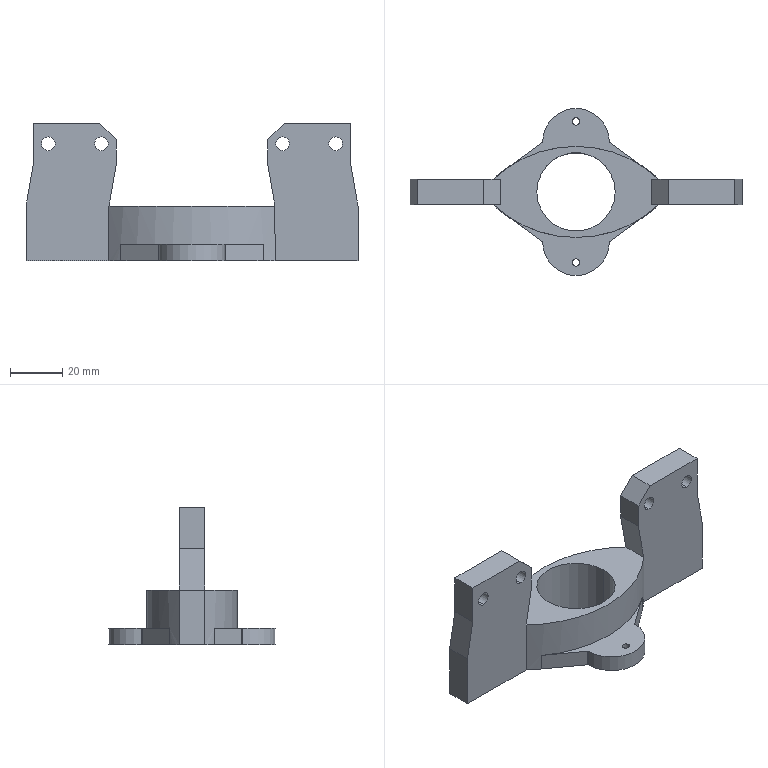Part | SolidWorks | features ICE 6, Chamfer 1, Cut 1, Extrusion 1, MirrorPattern 1 | 1 solid | 48 faces | box 127 x 64 x 52.75 mm | volume 56573 mm3 | plane 26 | cylinder 22 | commonest cylinder face diameters 5.207 x8 25.491 x6 2.8 x4 30 x2 92.779 x2
STEP:
#1=CARTESIAN_POINT('',(-34.666,4.826,21.209));
#2=VERTEX_POINT('',#1);
#3=CARTESIAN_POINT('',(-34.666,4.826,26.416));
#4=VERTEX_POINT('',#3);
#5=CARTESIAN_POINT('',(-34.666,4.826,23.812));
#6=DIRECTION('',(0.,1.,0.));
#7=DIRECTION('',(0.,0.,-1.));
#8=AXIS2_PLACEMENT_3D('',#5,#6,#7);
#9=CIRCLE('',#8,2.604);
#10=EDGE_CURVE('',#2,#4,#9,.T.);
#11=ORIENTED_EDGE('',*,*,#10,.T.);
#12=CARTESIAN_POINT('',(-34.666,-4.826,26.416));
#13=VERTEX_POINT('',#12);
#14=CARTESIAN_POINT('',(-34.666,51.748,26.416));
#15=DIRECTION('',(0.,-1.,0.));
#16=VECTOR('',#15,1000.);
#17=LINE('',#14,#16);
#18=EDGE_CURVE('',#4,#13,#17,.T.);
#19=ORIENTED_EDGE('',*,*,#18,.T.);
#20=CARTESIAN_POINT('',(-34.666,-4.826,21.209));
#21=VERTEX_POINT('',#20);
#22=CARTESIAN_POINT('',(-34.666,-4.826,23.812));
#23=DIRECTION('',(0.,-1.,0.));
#24=DIRECTION('',(0.,0.,-1.));
#25=AXIS2_PLACEMENT_3D('',#22,#23,#24);
#26=CIRCLE('',#25,2.604);
#27=EDGE_CURVE('',#13,#21,#26,.T.);
#28=ORIENTED_EDGE('',*,*,#27,.T.);
#29=CARTESIAN_POINT('',(-34.666,51.748,21.209));
#30=DIRECTION('',(0.,-1.,0.));
#31=VECTOR('',#30,1000.);
#32=LINE('',#29,#31);
#33=EDGE_CURVE('',#2,#21,#32,.T.);
#34=ORIENTED_EDGE('',*,*,#33,.F.);
#35=EDGE_LOOP('',(#11,#19,#28,#34));
#36=FACE_OUTER_BOUND('',#35,.T.);
#37=CARTESIAN_POINT('',(-34.666,51.748,23.812));
#38=DIRECTION('',(0.,-1.,0.));
#39=DIRECTION('',(0.,0.,-1.));
#40=AXIS2_PLACEMENT_3D('',#37,#38,#39);
#41=CYLINDRICAL_SURFACE('',#40,2.604);
#42=ADVANCED_FACE('',(#36),#41,.F.);
#43=CARTESIAN_POINT('',(-54.986,4.826,21.209));
#44=VERTEX_POINT('',#43);
#45=CARTESIAN_POINT('',(-54.986,4.826,26.416));
#46=VERTEX_POINT('',#45);
#47=CARTESIAN_POINT('',(-54.986,4.826,23.812));
#48=DIRECTION('',(0.,1.,0.));
#49=DIRECTION('',(0.,0.,-1.));
#50=AXIS2_PLACEMENT_3D('',#47,#48,#49);
#51=CIRCLE('',#50,2.604);
#52=EDGE_CURVE('',#44,#46,#51,.T.);
#53=ORIENTED_EDGE('',*,*,#52,.T.);
#54=CARTESIAN_POINT('',(-54.986,-4.826,26.416));
#55=VERTEX_POINT('',#54);
#56=CARTESIAN_POINT('',(-54.986,51.748,26.416));
#57=DIRECTION('',(0.,-1.,0.));
#58=VECTOR('',#57,1000.);
#59=LINE('',#56,#58);
#60=EDGE_CURVE('',#46,#55,#59,.T.);
#61=ORIENTED_EDGE('',*,*,#60,.T.);
#62=CARTESIAN_POINT('',(-54.986,-4.826,21.209));
#63=VERTEX_POINT('',#62);
#64=CARTESIAN_POINT('',(-54.986,-4.826,23.812));
#65=DIRECTION('',(0.,-1.,0.));
#66=DIRECTION('',(0.,0.,-1.));
#67=AXIS2_PLACEMENT_3D('',#64,#65,#66);
#68=CIRCLE('',#67,2.604);
#69=EDGE_CURVE('',#55,#63,#68,.T.);
#70=ORIENTED_EDGE('',*,*,#69,.T.);
#71=CARTESIAN_POINT('',(-54.986,51.748,21.209));
#72=DIRECTION('',(0.,-1.,0.));
#73=VECTOR('',#72,1000.);
#74=LINE('',#71,#73);
#75=EDGE_CURVE('',#44,#63,#74,.T.);
#76=ORIENTED_EDGE('',*,*,#75,.F.);
#77=EDGE_LOOP('',(#53,#61,#70,#76));
#78=FACE_OUTER_BOUND('',#77,.T.);
#79=CARTESIAN_POINT('',(-54.986,51.748,23.812));
#80=DIRECTION('',(0.,-1.,0.));
#81=DIRECTION('',(0.,0.,-1.));
#82=AXIS2_PLACEMENT_3D('',#79,#80,#81);
#83=CYLINDRICAL_SURFACE('',#82,2.604);
#84=ADVANCED_FACE('',(#78),#83,.F.);
#85=CARTESIAN_POINT('',(54.986,4.826,26.416));
#86=VERTEX_POINT('',#85);
#87=CARTESIAN_POINT('',(54.986,4.826,21.209));
#88=VERTEX_POINT('',#87);
#89=CARTESIAN_POINT('',(54.986,4.826,23.812));
#90=DIRECTION('',(0.,-1.,0.));
#91=DIRECTION('',(0.,0.,-1.));
#92=AXIS2_PLACEMENT_3D('',#89,#90,#91);
#93=CIRCLE('',#92,2.603);
#94=EDGE_CURVE('',#86,#88,#93,.T.);
#95=ORIENTED_EDGE('',*,*,#94,.F.);
#96=CARTESIAN_POINT('',(54.986,-4.826,26.416));
#97=VERTEX_POINT('',#96);
#98=CARTESIAN_POINT('',(54.986,51.748,26.416));
#99=DIRECTION('',(0.,-1.,0.));
#100=VECTOR('',#99,1000.);
#101=LINE('',#98,#100);
#102=EDGE_CURVE('',#86,#97,#101,.T.);
#103=ORIENTED_EDGE('',*,*,#102,.T.);
#104=CARTESIAN_POINT('',(54.986,-4.826,21.209));
#105=VERTEX_POINT('',#104);
#106=CARTESIAN_POINT('',(54.986,-4.826,23.812));
#107=DIRECTION('',(0.,1.,0.));
#108=DIRECTION('',(0.,0.,-1.));
#109=AXIS2_PLACEMENT_3D('',#106,#107,#108);
#110=CIRCLE('',#109,2.603);
#111=EDGE_CURVE('',#105,#97,#110,.T.);
#112=ORIENTED_EDGE('',*,*,#111,.F.);
#113=CARTESIAN_POINT('',(54.986,51.748,21.209));
#114=DIRECTION('',(0.,-1.,0.));
#115=VECTOR('',#114,1000.);
#116=LINE('',#113,#115);
#117=EDGE_CURVE('',#88,#105,#116,.T.);
#118=ORIENTED_EDGE('',*,*,#117,.F.);
#119=EDGE_LOOP('',(#95,#103,#112,#118));
#120=FACE_OUTER_BOUND('',#119,.T.);
#121=CARTESIAN_POINT('',(54.986,51.748,23.812));
#122=DIRECTION('',(0.,-1.,0.));
#123=DIRECTION('',(0.,0.,-1.));
#124=AXIS2_PLACEMENT_3D('',#121,#122,#123);
#125=CYLINDRICAL_SURFACE('',#124,2.603);
#126=ADVANCED_FACE('',(#120),#125,.F.);
#127=CARTESIAN_POINT('',(34.666,4.826,26.416));
#128=VERTEX_POINT('',#127);
#129=CARTESIAN_POINT('',(34.666,4.826,21.209));
#130=VERTEX_POINT('',#129);
#131=CARTESIAN_POINT('',(34.666,4.826,23.812));
#132=DIRECTION('',(0.,-1.,0.));
#133=DIRECTION('',(0.,0.,-1.));
#134=AXIS2_PLACEMENT_3D('',#131,#132,#133);
#135=CIRCLE('',#134,2.603);
#136=EDGE_CURVE('',#128,#130,#135,.T.);
#137=ORIENTED_EDGE('',*,*,#136,.F.);
#138=CARTESIAN_POINT('',(34.666,-4.826,26.416));
#139=VERTEX_POINT('',#138);
#140=CARTESIAN_POINT('',(34.666,51.748,26.416));
#141=DIRECTION('',(0.,-1.,0.));
#142=VECTOR('',#141,1000.);
#143=LINE('',#140,#142);
#144=EDGE_CURVE('',#128,#139,#143,.T.);
#145=ORIENTED_EDGE('',*,*,#144,.T.);
#146=CARTESIAN_POINT('',(34.666,-4.826,21.209));
#147=VERTEX_POINT('',#146);
#148=CARTESIAN_POINT('',(34.666,-4.826,23.812));
#149=DIRECTION('',(0.,1.,0.));
#150=DIRECTION('',(0.,0.,-1.));
#151=AXIS2_PLACEMENT_3D('',#148,#149,#150);
#152=CIRCLE('',#151,2.603);
#153=EDGE_CURVE('',#147,#139,#152,.T.);
#154=ORIENTED_EDGE('',*,*,#153,.F.);
#155=CARTESIAN_POINT('',(34.666,51.748,21.209));
#156=DIRECTION('',(0.,-1.,0.));
#157=VECTOR('',#156,1000.);
#158=LINE('',#155,#157);
#159=EDGE_CURVE('',#130,#147,#158,.T.);
#160=ORIENTED_EDGE('',*,*,#159,.F.);
#161=EDGE_LOOP('',(#137,#145,#154,#160));
#162=FACE_OUTER_BOUND('',#161,.T.);
#163=CARTESIAN_POINT('',(34.666,51.748,23.812));
#164=DIRECTION('',(0.,-1.,0.));
#165=DIRECTION('',(0.,0.,-1.));
#166=AXIS2_PLACEMENT_3D('',#163,#164,#165);
#167=CYLINDRICAL_SURFACE('',#166,2.603);
#168=ADVANCED_FACE('',(#162),#167,.F.);
#169=CARTESIAN_POINT('',(1.4,27.,-21.));
#170=VERTEX_POINT('',#169);
#171=CARTESIAN_POINT('',(-1.4,27.,-21.));
#172=VERTEX_POINT('',#171);
#173=CARTESIAN_POINT('',(0.,27.,-21.));
#174=DIRECTION('',(0.,0.,-1.));
#175=DIRECTION('',(1.,0.,0.));
#176=AXIS2_PLACEMENT_3D('',#173,#174,#175);
#177=CIRCLE('',#176,1.4);
#178=EDGE_CURVE('',#170,#172,#177,.T.);
#179=ORIENTED_EDGE('',*,*,#178,.T.);
#180=CARTESIAN_POINT('',(-1.4,27.,-14.65));
#181=VERTEX_POINT('',#180);
#182=CARTESIAN_POINT('',(-1.4,27.,-21.));
#183=DIRECTION('',(0.,0.,1.));
#184=VECTOR('',#183,1000.);
#185=LINE('',#182,#184);
#186=EDGE_CURVE('',#172,#181,#185,.T.);
#187=ORIENTED_EDGE('',*,*,#186,.T.);
#188=CARTESIAN_POINT('',(1.4,27.,-14.65));
#189=VERTEX_POINT('',#188);
#190=CARTESIAN_POINT('',(0.,27.,-14.65));
#191=DIRECTION('',(0.,0.,-1.));
#192=DIRECTION('',(1.,0.,0.));
#193=AXIS2_PLACEMENT_3D('',#190,#191,#192);
#194=CIRCLE('',#193,1.4);
#195=EDGE_CURVE('',#189,#181,#194,.T.);
#196=ORIENTED_EDGE('',*,*,#195,.F.);
#197=CARTESIAN_POINT('',(1.4,27.,-21.));
#198=DIRECTION('',(0.,0.,1.));
#199=VECTOR('',#198,1000.);
#200=LINE('',#197,#199);
#201=EDGE_CURVE('',#170,#189,#200,.T.);
#202=ORIENTED_EDGE('',*,*,#201,.F.);
#203=EDGE_LOOP('',(#179,#187,#196,#202));
#204=FACE_OUTER_BOUND('',#203,.T.);
#205=CARTESIAN_POINT('',(0.,27.,-21.));
#206=DIRECTION('',(0.,0.,1.));
#207=DIRECTION('',(1.,0.,0.));
#208=AXIS2_PLACEMENT_3D('',#205,#206,#207);
#209=CYLINDRICAL_SURFACE('',#208,1.4);
#210=ADVANCED_FACE('',(#204),#209,.F.);
#211=CARTESIAN_POINT('',(-12.745,19.255,-14.65));
#212=VERTEX_POINT('',#211);
#213=CARTESIAN_POINT('',(12.745,19.255,-14.65));
#214=VERTEX_POINT('',#213);
#215=CARTESIAN_POINT('',(0.,19.255,-14.65));
#216=DIRECTION('',(0.,0.,-1.));
#217=DIRECTION('',(-1.,0.,0.));
#218=AXIS2_PLACEMENT_3D('',#215,#216,#217);
#219=CIRCLE('',#218,12.745);
#220=EDGE_CURVE('',#212,#214,#219,.T.);
#221=ORIENTED_EDGE('',*,*,#220,.T.);
#222=CARTESIAN_POINT('',(12.745,19.255,-21.));
#223=VERTEX_POINT('',#222);
#224=CARTESIAN_POINT('',(12.745,19.255,-14.65));
#225=DIRECTION('',(0.,0.,-1.));
#226=VECTOR('',#225,1000.);
#227=LINE('',#224,#226);
#228=EDGE_CURVE('',#214,#223,#227,.T.);
#229=ORIENTED_EDGE('',*,*,#228,.T.);
#230=CARTESIAN_POINT('',(-12.745,19.255,-21.));
#231=VERTEX_POINT('',#230);
#232=CARTESIAN_POINT('',(0.,19.255,-21.));
#233=DIRECTION('',(0.,0.,-1.));
#234=DIRECTION('',(-1.,0.,0.));
#235=AXIS2_PLACEMENT_3D('',#232,#233,#234);
#236=CIRCLE('',#235,12.745);
#237=EDGE_CURVE('',#231,#223,#236,.T.);
#238=ORIENTED_EDGE('',*,*,#237,.F.);
#239=CARTESIAN_POINT('',(-12.745,19.255,-14.65));
#240=DIRECTION('',(0.,0.,-1.));
#241=VECTOR('',#240,1000.);
#242=LINE('',#239,#241);
#243=EDGE_CURVE('',#212,#231,#242,.T.);
#244=ORIENTED_EDGE('',*,*,#243,.F.);
#245=EDGE_LOOP('',(#221,#229,#238,#244));
#246=FACE_OUTER_BOUND('',#245,.T.);
#247=CARTESIAN_POINT('',(0.,19.255,-14.65));
#248=DIRECTION('',(0.,0.,-1.));
#249=DIRECTION('',(-1.,0.,0.));
#250=AXIS2_PLACEMENT_3D('',#247,#248,#249);
#251=CYLINDRICAL_SURFACE('',#250,12.745);
#252=ADVANCED_FACE('',(#246),#251,.T.);
#253=CARTESIAN_POINT('',(-12.744,19.05,-14.65));
#254=VERTEX_POINT('',#253);
#255=CARTESIAN_POINT('',(0.,19.255,-14.65));
#256=DIRECTION('',(0.,0.,-1.));
#257=DIRECTION('',(-1.,0.,0.));
#258=AXIS2_PLACEMENT_3D('',#255,#256,#257);
#259=CIRCLE('',#258,12.745);
#260=EDGE_CURVE('',#254,#212,#259,.T.);
#261=ORIENTED_EDGE('',*,*,#260,.T.);
#262=ORIENTED_EDGE('',*,*,#243,.T.);
#263=CARTESIAN_POINT('',(-12.744,19.05,-21.));
#264=VERTEX_POINT('',#263);
#265=CARTESIAN_POINT('',(0.,19.255,-21.));
#266=DIRECTION('',(0.,0.,-1.));
#267=DIRECTION('',(-1.,0.,0.));
#268=AXIS2_PLACEMENT_3D('',#265,#266,#267);
#269=CIRCLE('',#268,12.745);
#270=EDGE_CURVE('',#264,#231,#269,.T.);
#271=ORIENTED_EDGE('',*,*,#270,.F.);
#272=CARTESIAN_POINT('',(-12.744,19.05,-14.65));
#273=DIRECTION('',(0.,0.,-1.));
#274=VECTOR('',#273,1000.);
#275=LINE('',#272,#274);
#276=EDGE_CURVE('',#254,#264,#275,.T.);
#277=ORIENTED_EDGE('',*,*,#276,.F.);
#278=EDGE_LOOP('',(#261,#262,#271,#277));
#279=FACE_OUTER_BOUND('',#278,.T.);
#280=CARTESIAN_POINT('',(0.,19.255,-14.65));
#281=DIRECTION('',(0.,0.,-1.));
#282=DIRECTION('',(-1.,0.,0.));
#283=AXIS2_PLACEMENT_3D('',#280,#281,#282);
#284=CYLINDRICAL_SURFACE('',#283,12.745);
#285=ADVANCED_FACE('',(#279),#284,.T.);
#286=CARTESIAN_POINT('',(-1.4,-27.,-21.));
#287=VERTEX_POINT('',#286);
#288=CARTESIAN_POINT('',(1.4,-27.,-21.));
#289=VERTEX_POINT('',#288);
#290=CARTESIAN_POINT('',(0.,-27.,-21.));
#291=DIRECTION('',(0.,0.,1.));
#292=DIRECTION('',(1.,0.,0.));
#293=AXIS2_PLACEMENT_3D('',#290,#291,#292);
#294=CIRCLE('',#293,1.4);
#295=EDGE_CURVE('',#287,#289,#294,.T.);
#296=ORIENTED_EDGE('',*,*,#295,.F.);
#297=CARTESIAN_POINT('',(-1.4,-27.,-14.65));
#298=VERTEX_POINT('',#297);
#299=CARTESIAN_POINT('',(-1.4,-27.,-21.));
#300=DIRECTION('',(0.,0.,1.));
#301=VECTOR('',#300,1000.);
#302=LINE('',#299,#301);
#303=EDGE_CURVE('',#287,#298,#302,.T.);
#304=ORIENTED_EDGE('',*,*,#303,.T.);
#305=CARTESIAN_POINT('',(1.4,-27.,-14.65));
#306=VERTEX_POINT('',#305);
#307=CARTESIAN_POINT('',(0.,-27.,-14.65));
#308=DIRECTION('',(0.,0.,1.));
#309=DIRECTION('',(1.,0.,0.));
#310=AXIS2_PLACEMENT_3D('',#307,#308,#309);
#311=CIRCLE('',#310,1.4);
#312=EDGE_CURVE('',#298,#306,#311,.T.);
#313=ORIENTED_EDGE('',*,*,#312,.T.);
#314=CARTESIAN_POINT('',(1.4,-27.,-21.));
#315=DIRECTION('',(0.,0.,1.));
#316=VECTOR('',#315,1000.);
#317=LINE('',#314,#316);
#318=EDGE_CURVE('',#289,#306,#317,.T.);
#319=ORIENTED_EDGE('',*,*,#318,.F.);
#320=EDGE_LOOP('',(#296,#304,#313,#319));
#321=FACE_OUTER_BOUND('',#320,.T.);
#322=CARTESIAN_POINT('',(0.,-27.,-21.));
#323=DIRECTION('',(0.,0.,1.));
#324=DIRECTION('',(1.,0.,0.));
#325=AXIS2_PLACEMENT_3D('',#322,#323,#324);
#326=CYLINDRICAL_SURFACE('',#325,1.4);
#327=ADVANCED_FACE('',(#321),#326,.F.);
#328=CARTESIAN_POINT('',(12.745,-19.255,-14.65));
#329=VERTEX_POINT('',#328);
#330=CARTESIAN_POINT('',(12.744,-19.05,-14.65));
#331=VERTEX_POINT('',#330);
#332=CARTESIAN_POINT('',(0.,-19.255,-14.65));
#333=DIRECTION('',(0.,0.,1.));
#334=DIRECTION('',(-1.,0.,0.));
#335=AXIS2_PLACEMENT_3D('',#332,#333,#334);
#336=CIRCLE('',#335,12.745);
#337=EDGE_CURVE('',#329,#331,#336,.T.);
#338=ORIENTED_EDGE('',*,*,#337,.F.);
#339=CARTESIAN_POINT('',(12.745,-19.255,-21.));
#340=VERTEX_POINT('',#339);
#341=CARTESIAN_POINT('',(12.745,-19.255,-14.65));
#342=DIRECTION('',(0.,0.,-1.));
#343=VECTOR('',#342,1000.);
#344=LINE('',#341,#343);
#345=EDGE_CURVE('',#329,#340,#344,.T.);
#346=ORIENTED_EDGE('',*,*,#345,.T.);
#347=CARTESIAN_POINT('',(12.744,-19.05,-21.));
#348=VERTEX_POINT('',#347);
#349=CARTESIAN_POINT('',(0.,-19.255,-21.));
#350=DIRECTION('',(0.,0.,1.));
#351=DIRECTION('',(-1.,0.,0.));
#352=AXIS2_PLACEMENT_3D('',#349,#350,#351);
#353=CIRCLE('',#352,12.745);
#354=EDGE_CURVE('',#340,#348,#353,.T.);
#355=ORIENTED_EDGE('',*,*,#354,.T.);
#356=CARTESIAN_POINT('',(12.744,-19.05,-14.65));
#357=DIRECTION('',(0.,0.,-1.));
#358=VECTOR('',#357,1000.);
#359=LINE('',#356,#358);
#360=EDGE_CURVE('',#331,#348,#359,.T.);
#361=ORIENTED_EDGE('',*,*,#360,.F.);
#362=EDGE_LOOP('',(#338,#346,#355,#361));
#363=FACE_OUTER_BOUND('',#362,.T.);
#364=CARTESIAN_POINT('',(0.,-19.255,-14.65));
#365=DIRECTION('',(0.,0.,-1.));
#366=DIRECTION('',(-1.,0.,0.));
#367=AXIS2_PLACEMENT_3D('',#364,#365,#366);
#368=CYLINDRICAL_SURFACE('',#367,12.745);
#369=ADVANCED_FACE('',(#363),#368,.T.);
#370=ORIENTED_EDGE('',*,*,#345,.F.);
#371=CARTESIAN_POINT('',(-12.745,-19.255,-14.65));
#372=VERTEX_POINT('',#371);
#373=CARTESIAN_POINT('',(0.,-19.255,-14.65));
#374=DIRECTION('',(0.,0.,1.));
#375=DIRECTION('',(-1.,0.,0.));
#376=AXIS2_PLACEMENT_3D('',#373,#374,#375);
#377=CIRCLE('',#376,12.745);
#378=EDGE_CURVE('',#372,#329,#377,.T.);
#379=ORIENTED_EDGE('',*,*,#378,.F.);
#380=CARTESIAN_POINT('',(-12.745,-19.255,-21.));
#381=VERTEX_POINT('',#380);
#382=CARTESIAN_POINT('',(-12.745,-19.255,-14.65));
#383=DIRECTION('',(0.,0.,-1.));
#384=VECTOR('',#383,1000.);
#385=LINE('',#382,#384);
#386=EDGE_CURVE('',#372,#381,#385,.T.);
#387=ORIENTED_EDGE('',*,*,#386,.T.);
#388=CARTESIAN_POINT('',(0.,-19.255,-21.));
#389=DIRECTION('',(0.,0.,1.));
#390=DIRECTION('',(-1.,0.,0.));
#391=AXIS2_PLACEMENT_3D('',#388,#389,#390);
#392=CIRCLE('',#391,12.745);
#393=EDGE_CURVE('',#381,#340,#392,.T.);
#394=ORIENTED_EDGE('',*,*,#393,.T.);
#395=EDGE_LOOP('',(#370,#379,#387,#394));
#396=FACE_OUTER_BOUND('',#395,.T.);
#397=CARTESIAN_POINT('',(0.,-19.255,-14.65));
#398=DIRECTION('',(0.,0.,-1.));
#399=DIRECTION('',(-1.,0.,0.));
#400=AXIS2_PLACEMENT_3D('',#397,#398,#399);
#401=CYLINDRICAL_SURFACE('',#400,12.745);
#402=ADVANCED_FACE('',(#396),#401,.T.);
#403=CARTESIAN_POINT('',(15.,0.,-21.));
#404=VERTEX_POINT('',#403);
#405=CARTESIAN_POINT('',(-15.,0.,-21.));
#406=VERTEX_POINT('',#405);
#407=CARTESIAN_POINT('',(0.,0.,-21.));
#408=DIRECTION('',(0.,0.,-1.));
#409=DIRECTION('',(1.,0.,0.));
#410=AXIS2_PLACEMENT_3D('',#407,#408,#409);
#411=CIRCLE('',#410,15.);
#412=EDGE_CURVE('',#404,#406,#411,.T.);
#413=ORIENTED_EDGE('',*,*,#412,.T.);
#414=CARTESIAN_POINT('',(-15.,0.,0.));
#415=VERTEX_POINT('',#414);
#416=CARTESIAN_POINT('',(-15.,0.,-153.592));
#417=DIRECTION('',(0.,0.,1.));
#418=VECTOR('',#417,1000.);
#419=LINE('',#416,#418);
#420=EDGE_CURVE('',#406,#415,#419,.T.);
#421=ORIENTED_EDGE('',*,*,#420,.T.);
#422=CARTESIAN_POINT('',(15.,0.,0.));
#423=VERTEX_POINT('',#422);
#424=CARTESIAN_POINT('',(0.,0.,0.));
#425=DIRECTION('',(0.,0.,1.));
#426=DIRECTION('',(1.,0.,0.));
#427=AXIS2_PLACEMENT_3D('',#424,#425,#426);
#428=CIRCLE('',#427,15.);
#429=EDGE_CURVE('',#415,#423,#428,.T.);
#430=ORIENTED_EDGE('',*,*,#429,.T.);
#431=CARTESIAN_POINT('',(15.,0.,-153.592));
#432=DIRECTION('',(0.,0.,1.));
#433=VECTOR('',#432,1000.);
#434=LINE('',#431,#433);
#435=EDGE_CURVE('',#404,#423,#434,.T.);
#436=ORIENTED_EDGE('',*,*,#435,.F.);
#437=EDGE_LOOP('',(#413,#421,#430,#436));
#438=FACE_OUTER_BOUND('',#437,.T.);
#439=CARTESIAN_POINT('',(0.,0.,-153.592));
#440=DIRECTION('',(0.,0.,1.));
#441=DIRECTION('',(1.,0.,0.));
#442=AXIS2_PLACEMENT_3D('',#439,#440,#441);
#443=CYLINDRICAL_SURFACE('',#442,15.);
#444=ADVANCED_FACE('',(#438),#443,.F.);
#445=CARTESIAN_POINT('',(0.,0.,0.));
#446=DIRECTION('',(0.,0.,1.));
#447=DIRECTION('',(1.,0.,0.));
#448=AXIS2_PLACEMENT_3D('',#445,#446,#447);
#449=CIRCLE('',#448,15.);
#450=EDGE_CURVE('',#423,#415,#449,.T.);
#451=ORIENTED_EDGE('',*,*,#450,.F.);
#452=ORIENTED_EDGE('',*,*,#429,.F.);
#453=EDGE_LOOP('',(#451,#452));
#454=FACE_BOUND('',#453,.T.);
#455=CARTESIAN_POINT('',(31.75,4.826,0.));
#456=VERTEX_POINT('',#455);
#457=CARTESIAN_POINT('',(-31.75,4.826,0.));
#458=VERTEX_POINT('',#457);
#459=CARTESIAN_POINT('',(0.,-28.996,0.));
#460=DIRECTION('',(0.,0.,1.));
#461=DIRECTION('',(1.,0.,0.));
#462=AXIS2_PLACEMENT_3D('',#459,#460,#461);
#463=CIRCLE('',#462,46.39);
#464=EDGE_CURVE('',#456,#458,#463,.T.);
#465=ORIENTED_EDGE('',*,*,#464,.T.);
#466=CARTESIAN_POINT('',(-31.75,-4.826,0.));
#467=VERTEX_POINT('',#466);
#468=CARTESIAN_POINT('',(-31.75,51.748,0.));
#469=DIRECTION('',(0.,-1.,0.));
#470=VECTOR('',#469,1000.);
#471=LINE('',#468,#470);
#472=EDGE_CURVE('',#458,#467,#471,.T.);
#473=ORIENTED_EDGE('',*,*,#472,.T.);
#474=CARTESIAN_POINT('',(31.75,-4.826,0.));
#475=VERTEX_POINT('',#474);
#476=CARTESIAN_POINT('',(0.,28.996,0.));
#477=DIRECTION('',(0.,0.,-1.));
#478=DIRECTION('',(1.,0.,0.));
#479=AXIS2_PLACEMENT_3D('',#476,#477,#478);
#480=CIRCLE('',#479,46.39);
#481=EDGE_CURVE('',#475,#467,#480,.T.);
#482=ORIENTED_EDGE('',*,*,#481,.F.);
#483=CARTESIAN_POINT('',(31.75,51.748,0.));
#484=DIRECTION('',(0.,-1.,0.));
#485=VECTOR('',#484,1000.);
#486=LINE('',#483,#485);
#487=EDGE_CURVE('',#456,#475,#486,.T.);
#488=ORIENTED_EDGE('',*,*,#487,.F.);
#489=EDGE_LOOP('',(#465,#473,#482,#488));
#490=FACE_OUTER_BOUND('',#489,.T.);
#491=CARTESIAN_POINT('',(0.,0.,0.));
#492=DIRECTION('',(0.,0.,1.));
#493=DIRECTION('',(1.,0.,0.));
#494=AXIS2_PLACEMENT_3D('',#491,#492,#493);
#495=PLANE('',#494);
#496=ADVANCED_FACE('',(#454,#490),#495,.T.);
#497=ORIENTED_EDGE('',*,*,#412,.F.);
#498=CARTESIAN_POINT('',(0.,0.,-21.));
#499=DIRECTION('',(0.,0.,-1.));
#500=DIRECTION('',(1.,0.,0.));
#501=AXIS2_PLACEMENT_3D('',#498,#499,#500);
#502=CIRCLE('',#501,15.);
#503=EDGE_CURVE('',#406,#404,#502,.T.);
#504=ORIENTED_EDGE('',*,*,#503,.F.);
#505=EDGE_LOOP('',(#497,#504));
#506=FACE_BOUND('',#505,.T.);
#507=CARTESIAN_POINT('',(0.,-27.,-21.));
#508=DIRECTION('',(0.,0.,1.));
#509=DIRECTION('',(1.,0.,0.));
#510=AXIS2_PLACEMENT_3D('',#507,#508,#509);
#511=CIRCLE('',#510,1.4);
#512=EDGE_CURVE('',#289,#287,#511,.T.);
#513=ORIENTED_EDGE('',*,*,#512,.T.);
#514=ORIENTED_EDGE('',*,*,#295,.T.);
#515=EDGE_LOOP('',(#513,#514));
#516=FACE_BOUND('',#515,.T.);
#517=ORIENTED_EDGE('',*,*,#178,.F.);
#518=CARTESIAN_POINT('',(0.,27.,-21.));
#519=DIRECTION('',(0.,0.,-1.));
#520=DIRECTION('',(1.,0.,0.));
#521=AXIS2_PLACEMENT_3D('',#518,#519,#520);
#522=CIRCLE('',#521,1.4);
#523=EDGE_CURVE('',#172,#170,#522,.T.);
#524=ORIENTED_EDGE('',*,*,#523,.F.);
#525=EDGE_LOOP('',(#517,#524));
#526=FACE_BOUND('',#525,.T.);
#527=CARTESIAN_POINT('',(27.206,-8.578,-21.));
#528=VERTEX_POINT('',#527);
#529=CARTESIAN_POINT('',(13.433,-18.551,-21.));
#530=DIRECTION('',(0.81,0.5865,0.));
#531=VECTOR('',#530,1000.);
#532=LINE('',#529,#531);
#533=EDGE_CURVE('',#348,#528,#532,.T.);
#534=ORIENTED_EDGE('',*,*,#533,.F.);
#535=ORIENTED_EDGE('',*,*,#354,.F.);
#536=ORIENTED_EDGE('',*,*,#393,.F.);
#537=CARTESIAN_POINT('',(-12.744,-19.05,-21.));
#538=VERTEX_POINT('',#537);
#539=CARTESIAN_POINT('',(0.,-19.255,-21.));
#540=DIRECTION('',(0.,0.,1.));
#541=DIRECTION('',(-1.,0.,0.));
#542=AXIS2_PLACEMENT_3D('',#539,#540,#541);
#543=CIRCLE('',#542,12.745);
#544=EDGE_CURVE('',#538,#381,#543,.T.);
#545=ORIENTED_EDGE('',*,*,#544,.F.);
#546=CARTESIAN_POINT('',(-27.206,-8.578,-21.));
#547=VERTEX_POINT('',#546);
#548=CARTESIAN_POINT('',(-13.433,-18.551,-21.));
#549=DIRECTION('',(-0.81,0.5865,0.));
#550=VECTOR('',#549,1000.);
#551=LINE('',#548,#550);
#552=EDGE_CURVE('',#538,#547,#551,.T.);
#553=ORIENTED_EDGE('',*,*,#552,.T.);
#554=CARTESIAN_POINT('',(-31.75,-4.826,-21.));
#555=VERTEX_POINT('',#554);
#556=CARTESIAN_POINT('',(0.,28.996,-21.));
#557=DIRECTION('',(0.,0.,-1.));
#558=DIRECTION('',(1.,0.,0.));
#559=AXIS2_PLACEMENT_3D('',#556,#557,#558);
#560=CIRCLE('',#559,46.39);
#561=EDGE_CURVE('',#547,#555,#560,.T.);
#562=ORIENTED_EDGE('',*,*,#561,.T.);
#563=CARTESIAN_POINT('',(-63.5,-4.826,-21.));
#564=VERTEX_POINT('',#563);
#565=CARTESIAN_POINT('',(0.,-4.826,-21.));
#566=DIRECTION('',(-1.,0.,0.));
#567=VECTOR('',#566,1000.);
#568=LINE('',#565,#567);
#569=EDGE_CURVE('',#555,#564,#568,.T.);
#570=ORIENTED_EDGE('',*,*,#569,.T.);
#571=CARTESIAN_POINT('',(-63.5,4.826,-21.));
#572=VERTEX_POINT('',#571);
#573=CARTESIAN_POINT('',(-63.5,0.,-21.));
#574=DIRECTION('',(0.,-1.,0.));
#575=VECTOR('',#574,1000.);
#576=LINE('',#573,#575);
#577=EDGE_CURVE('',#572,#564,#576,.T.);
#578=ORIENTED_EDGE('',*,*,#577,.F.);
#579=CARTESIAN_POINT('',(-31.75,4.826,-21.));
#580=VERTEX_POINT('',#579);
#581=CARTESIAN_POINT('',(0.,4.826,-21.));
#582=DIRECTION('',(1.,0.,0.));
#583=VECTOR('',#582,1000.);
#584=LINE('',#581,#583);
#585=EDGE_CURVE('',#572,#580,#584,.T.);
#586=ORIENTED_EDGE('',*,*,#585,.T.);
#587=CARTESIAN_POINT('',(-27.206,8.578,-21.));
#588=VERTEX_POINT('',#587);
#589=CARTESIAN_POINT('',(0.,-28.996,-21.));
#590=DIRECTION('',(0.,0.,1.));
#591=DIRECTION('',(1.,0.,0.));
#592=AXIS2_PLACEMENT_3D('',#589,#590,#591);
#593=CIRCLE('',#592,46.39);
#594=EDGE_CURVE('',#588,#580,#593,.T.);
#595=ORIENTED_EDGE('',*,*,#594,.F.);
#596=CARTESIAN_POINT('',(-13.433,18.551,-21.));
#597=DIRECTION('',(-0.81,-0.5865,0.));
#598=VECTOR('',#597,1000.);
#599=LINE('',#596,#598);
#600=EDGE_CURVE('',#264,#588,#599,.T.);
#601=ORIENTED_EDGE('',*,*,#600,.F.);
#602=ORIENTED_EDGE('',*,*,#270,.T.);
#603=ORIENTED_EDGE('',*,*,#237,.T.);
#604=CARTESIAN_POINT('',(12.744,19.05,-21.));
#605=VERTEX_POINT('',#604);
#606=CARTESIAN_POINT('',(0.,19.255,-21.));
#607=DIRECTION('',(0.,0.,-1.));
#608=DIRECTION('',(-1.,0.,0.));
#609=AXIS2_PLACEMENT_3D('',#606,#607,#608);
#610=CIRCLE('',#609,12.745);
#611=EDGE_CURVE('',#223,#605,#610,.T.);
#612=ORIENTED_EDGE('',*,*,#611,.T.);
#613=CARTESIAN_POINT('',(27.206,8.578,-21.));
#614=VERTEX_POINT('',#613);
#615=CARTESIAN_POINT('',(13.433,18.551,-21.));
#616=DIRECTION('',(0.81,-0.5865,0.));
#617=VECTOR('',#616,1000.);
#618=LINE('',#615,#617);
#619=EDGE_CURVE('',#605,#614,#618,.T.);
#620=ORIENTED_EDGE('',*,*,#619,.T.);
#621=CARTESIAN_POINT('',(31.75,4.826,-21.));
#622=VERTEX_POINT('',#621);
#623=CARTESIAN_POINT('',(0.,-28.996,-21.));
#624=DIRECTION('',(0.,0.,1.));
#625=DIRECTION('',(1.,0.,0.));
#626=AXIS2_PLACEMENT_3D('',#623,#624,#625);
#627=CIRCLE('',#626,46.39);
#628=EDGE_CURVE('',#622,#614,#627,.T.);
#629=ORIENTED_EDGE('',*,*,#628,.F.);
#630=CARTESIAN_POINT('',(63.5,4.826,-21.));
#631=VERTEX_POINT('',#630);
#632=CARTESIAN_POINT('',(0.,4.826,-21.));
#633=DIRECTION('',(1.,0.,0.));
#634=VECTOR('',#633,1000.);
#635=LINE('',#632,#634);
#636=EDGE_CURVE('',#622,#631,#635,.T.);
#637=ORIENTED_EDGE('',*,*,#636,.T.);
#638=CARTESIAN_POINT('',(63.5,-4.826,-21.));
#639=VERTEX_POINT('',#638);
#640=CARTESIAN_POINT('',(63.5,0.,-21.));
#641=DIRECTION('',(0.,-1.,0.));
#642=VECTOR('',#641,1000.);
#643=LINE('',#640,#642);
#644=EDGE_CURVE('',#631,#639,#643,.T.);
#645=ORIENTED_EDGE('',*,*,#644,.T.);
#646=CARTESIAN_POINT('',(31.75,-4.826,-21.));
#647=VERTEX_POINT('',#646);
#648=CARTESIAN_POINT('',(0.,-4.826,-21.));
#649=DIRECTION('',(-1.,0.,0.));
#650=VECTOR('',#649,1000.);
#651=LINE('',#648,#650);
#652=EDGE_CURVE('',#639,#647,#651,.T.);
#653=ORIENTED_EDGE('',*,*,#652,.T.);
#654=CARTESIAN_POINT('',(0.,28.996,-21.));
#655=DIRECTION('',(0.,0.,-1.));
#656=DIRECTION('',(1.,0.,0.));
#657=AXIS2_PLACEMENT_3D('',#654,#655,#656);
#658=CIRCLE('',#657,46.39);
#659=EDGE_CURVE('',#647,#528,#658,.T.);
#660=ORIENTED_EDGE('',*,*,#659,.T.);
#661=EDGE_LOOP('',(#534,#535,#536,#545,#553,#562,#570,#578,#586,#595,#601,#602,#603,#612,#620,#629,#637,#645,#653,#660));
#662=FACE_OUTER_BOUND('',#661,.T.);
#663=CARTESIAN_POINT('',(0.,0.,-21.));
#664=DIRECTION('',(0.,0.,1.));
#665=DIRECTION('',(1.,0.,0.));
#666=AXIS2_PLACEMENT_3D('',#663,#664,#665);
#667=PLANE('',#666);
#668=ADVANCED_FACE('',(#506,#516,#526,#662),#667,.F.);
#669=CARTESIAN_POINT('',(0.,-27.,-14.65));
#670=DIRECTION('',(0.,0.,1.));
#671=DIRECTION('',(1.,0.,0.));
#672=AXIS2_PLACEMENT_3D('',#669,#670,#671);
#673=CIRCLE('',#672,1.4);
#674=EDGE_CURVE('',#306,#298,#673,.T.);
#675=ORIENTED_EDGE('',*,*,#674,.F.);
#676=ORIENTED_EDGE('',*,*,#312,.F.);
#677=EDGE_LOOP('',(#675,#676));
#678=FACE_BOUND('',#677,.T.);
#679=CARTESIAN_POINT('',(27.206,-8.578,-14.65));
#680=VERTEX_POINT('',#679);
#681=CARTESIAN_POINT('',(13.433,-18.551,-14.65));
#682=DIRECTION('',(0.81,0.5865,0.));
#683=VECTOR('',#682,1000.);
#684=LINE('',#681,#683);
#685=EDGE_CURVE('',#331,#680,#684,.T.);
#686=ORIENTED_EDGE('',*,*,#685,.T.);
#687=CARTESIAN_POINT('',(-27.206,-8.578,-14.65));
#688=VERTEX_POINT('',#687);
#689=CARTESIAN_POINT('',(0.,28.996,-14.65));
#690=DIRECTION('',(0.,0.,-1.));
#691=DIRECTION('',(-1.,0.,0.));
#692=AXIS2_PLACEMENT_3D('',#689,#690,#691);
#693=CIRCLE('',#692,46.39);
#694=EDGE_CURVE('',#680,#688,#693,.T.);
#695=ORIENTED_EDGE('',*,*,#694,.T.);
#696=CARTESIAN_POINT('',(-12.744,-19.05,-14.65));
#697=VERTEX_POINT('',#696);
#698=CARTESIAN_POINT('',(-13.433,-18.551,-14.65));
#699=DIRECTION('',(-0.81,0.5865,0.));
#700=VECTOR('',#699,1000.);
#701=LINE('',#698,#700);
#702=EDGE_CURVE('',#697,#688,#701,.T.);
#703=ORIENTED_EDGE('',*,*,#702,.F.);
#704=CARTESIAN_POINT('',(0.,-19.255,-14.65));
#705=DIRECTION('',(0.,0.,1.));
#706=DIRECTION('',(-1.,0.,0.));
#707=AXIS2_PLACEMENT_3D('',#704,#705,#706);
#708=CIRCLE('',#707,12.745);
#709=EDGE_CURVE('',#697,#372,#708,.T.);
#710=ORIENTED_EDGE('',*,*,#709,.T.);
#711=ORIENTED_EDGE('',*,*,#378,.T.);
#712=ORIENTED_EDGE('',*,*,#337,.T.);
#713=EDGE_LOOP('',(#686,#695,#703,#710,#711,#712));
#714=FACE_OUTER_BOUND('',#713,.T.);
#715=CARTESIAN_POINT('',(0.,0.,-14.65));
#716=DIRECTION('',(0.,0.,-1.));
#717=DIRECTION('',(-1.,0.,0.));
#718=AXIS2_PLACEMENT_3D('',#715,#716,#717);
#719=PLANE('',#718);
#720=ADVANCED_FACE('',(#678,#714),#719,.F.);
#721=ORIENTED_EDGE('',*,*,#195,.T.);
#722=CARTESIAN_POINT('',(0.,27.,-14.65));
#723=DIRECTION('',(0.,0.,-1.));
#724=DIRECTION('',(1.,0.,0.));
#725=AXIS2_PLACEMENT_3D('',#722,#723,#724);
#726=CIRCLE('',#725,1.4);
#727=EDGE_CURVE('',#181,#189,#726,.T.);
#728=ORIENTED_EDGE('',*,*,#727,.T.);
#729=EDGE_LOOP('',(#721,#728));
#730=FACE_BOUND('',#729,.T.);
#731=CARTESIAN_POINT('',(27.206,8.578,-14.65));
#732=VERTEX_POINT('',#731);
#733=CARTESIAN_POINT('',(-27.206,8.578,-14.65));
#734=VERTEX_POINT('',#733);
#735=CARTESIAN_POINT('',(0.,-28.996,-14.65));
#736=DIRECTION('',(0.,0.,1.));
#737=DIRECTION('',(-1.,0.,0.));
#738=AXIS2_PLACEMENT_3D('',#735,#736,#737);
#739=CIRCLE('',#738,46.39);
#740=EDGE_CURVE('',#732,#734,#739,.T.);
#741=ORIENTED_EDGE('',*,*,#740,.F.);
#742=CARTESIAN_POINT('',(12.744,19.05,-14.65));
#743=VERTEX_POINT('',#742);
#744=CARTESIAN_POINT('',(13.433,18.551,-14.65));
#745=DIRECTION('',(0.81,-0.5865,0.));
#746=VECTOR('',#745,1000.);
#747=LINE('',#744,#746);
#748=EDGE_CURVE('',#743,#732,#747,.T.);
#749=ORIENTED_EDGE('',*,*,#748,.F.);
#750=CARTESIAN_POINT('',(0.,19.255,-14.65));
#751=DIRECTION('',(0.,0.,-1.));
#752=DIRECTION('',(-1.,0.,0.));
#753=AXIS2_PLACEMENT_3D('',#750,#751,#752);
#754=CIRCLE('',#753,12.745);
#755=EDGE_CURVE('',#214,#743,#754,.T.);
#756=ORIENTED_EDGE('',*,*,#755,.F.);
#757=ORIENTED_EDGE('',*,*,#220,.F.);
#758=ORIENTED_EDGE('',*,*,#260,.F.);
#759=CARTESIAN_POINT('',(-13.433,18.551,-14.65));
#760=DIRECTION('',(-0.81,-0.5865,0.));
#761=VECTOR('',#760,1000.);
#762=LINE('',#759,#761);
#763=EDGE_CURVE('',#254,#734,#762,.T.);
#764=ORIENTED_EDGE('',*,*,#763,.T.);
#765=EDGE_LOOP('',(#741,#749,#756,#757,#758,#764));
#766=FACE_OUTER_BOUND('',#765,.T.);
#767=CARTESIAN_POINT('',(0.,0.,-14.65));
#768=DIRECTION('',(0.,0.,-1.));
#769=DIRECTION('',(-1.,0.,0.));
#770=AXIS2_PLACEMENT_3D('',#767,#768,#769);
#771=PLANE('',#770);
#772=ADVANCED_FACE('',(#730,#766),#771,.F.);
#773=CARTESIAN_POINT('',(-63.5,4.826,0.));
#774=VERTEX_POINT('',#773);
#775=CARTESIAN_POINT('',(-63.5,4.826,-142.444));
#776=DIRECTION('',(0.,0.,1.));
#777=VECTOR('',#776,1000.);
#778=LINE('',#775,#777);
#779=EDGE_CURVE('',#572,#774,#778,.T.);
#780=ORIENTED_EDGE('',*,*,#779,.F.);
#781=ORIENTED_EDGE('',*,*,#577,.T.);
#782=CARTESIAN_POINT('',(-63.5,-4.826,0.));
#783=VERTEX_POINT('',#782);
#784=CARTESIAN_POINT('',(-63.5,-4.826,-142.444));
#785=DIRECTION('',(0.,0.,1.));
#786=VECTOR('',#785,1000.);
#787=LINE('',#784,#786);
#788=EDGE_CURVE('',#564,#783,#787,.T.);
#789=ORIENTED_EDGE('',*,*,#788,.T.);
#790=CARTESIAN_POINT('',(-63.5,0.,0.));
#791=DIRECTION('',(0.,1.,0.));
#792=VECTOR('',#791,1000.);
#793=LINE('',#790,#792);
#794=EDGE_CURVE('',#783,#774,#793,.T.);
#795=ORIENTED_EDGE('',*,*,#794,.T.);
#796=EDGE_LOOP('',(#780,#781,#789,#795));
#797=FACE_OUTER_BOUND('',#796,.T.);
#798=CARTESIAN_POINT('',(-63.5,0.,-153.592));
#799=DIRECTION('',(1.,0.,0.));
#800=DIRECTION('',(0.,0.,-1.));
#801=AXIS2_PLACEMENT_3D('',#798,#799,#800);
#802=PLANE('',#801);
#803=ADVANCED_FACE('',(#797),#802,.F.);
#804=ORIENTED_EDGE('',*,*,#420,.F.);
#805=ORIENTED_EDGE('',*,*,#503,.T.);
#806=ORIENTED_EDGE('',*,*,#435,.T.);
#807=ORIENTED_EDGE('',*,*,#450,.T.);
#808=EDGE_LOOP('',(#804,#805,#806,#807));
#809=FACE_OUTER_BOUND('',#808,.T.);
#810=CARTESIAN_POINT('',(0.,0.,-153.592));
#811=DIRECTION('',(0.,0.,1.));
#812=DIRECTION('',(1.,0.,0.));
#813=AXIS2_PLACEMENT_3D('',#810,#811,#812);
#814=CYLINDRICAL_SURFACE('',#813,15.);
#815=ADVANCED_FACE('',(#809),#814,.F.);
#816=CARTESIAN_POINT('',(63.5,-4.826,0.));
#817=VERTEX_POINT('',#816);
#818=CARTESIAN_POINT('',(63.5,-4.826,-142.444));
#819=DIRECTION('',(0.,0.,1.));
#820=VECTOR('',#819,1000.);
#821=LINE('',#818,#820);
#822=EDGE_CURVE('',#639,#817,#821,.T.);
#823=ORIENTED_EDGE('',*,*,#822,.F.);
#824=ORIENTED_EDGE('',*,*,#644,.F.);
#825=CARTESIAN_POINT('',(63.5,4.826,0.));
#826=VERTEX_POINT('',#825);
#827=CARTESIAN_POINT('',(63.5,4.826,-142.444));
#828=DIRECTION('',(0.,0.,1.));
#829=VECTOR('',#828,1000.);
#830=LINE('',#827,#829);
#831=EDGE_CURVE('',#631,#826,#830,.T.);
#832=ORIENTED_EDGE('',*,*,#831,.T.);
#833=CARTESIAN_POINT('',(63.5,0.,0.));
#834=DIRECTION('',(0.,1.,0.));
#835=VECTOR('',#834,1000.);
#836=LINE('',#833,#835);
#837=EDGE_CURVE('',#817,#826,#836,.T.);
#838=ORIENTED_EDGE('',*,*,#837,.F.);
#839=EDGE_LOOP('',(#823,#824,#832,#838));
#840=FACE_OUTER_BOUND('',#839,.T.);
#841=CARTESIAN_POINT('',(63.5,0.,-153.592));
#842=DIRECTION('',(1.,0.,0.));
#843=DIRECTION('',(0.,0.,-1.));
#844=AXIS2_PLACEMENT_3D('',#841,#842,#843);
#845=PLANE('',#844);
#846=ADVANCED_FACE('',(#840),#845,.T.);
#847=ORIENTED_EDGE('',*,*,#386,.F.);
#848=ORIENTED_EDGE('',*,*,#709,.F.);
#849=CARTESIAN_POINT('',(-12.744,-19.05,-14.65));
#850=DIRECTION('',(0.,0.,-1.));
#851=VECTOR('',#850,1000.);
#852=LINE('',#849,#851);
#853=EDGE_CURVE('',#697,#538,#852,.T.);
#854=ORIENTED_EDGE('',*,*,#853,.T.);
#855=ORIENTED_EDGE('',*,*,#544,.T.);
#856=EDGE_LOOP('',(#847,#848,#854,#855));
#857=FACE_OUTER_BOUND('',#856,.T.);
#858=CARTESIAN_POINT('',(0.,-19.255,-14.65));
#859=DIRECTION('',(0.,0.,-1.));
#860=DIRECTION('',(-1.,0.,0.));
#861=AXIS2_PLACEMENT_3D('',#858,#859,#860);
#862=CYLINDRICAL_SURFACE('',#861,12.745);
#863=ADVANCED_FACE('',(#857),#862,.T.);
#864=ORIENTED_EDGE('',*,*,#303,.F.);
#865=ORIENTED_EDGE('',*,*,#512,.F.);
#866=ORIENTED_EDGE('',*,*,#318,.T.);
#867=ORIENTED_EDGE('',*,*,#674,.T.);
#868=EDGE_LOOP('',(#864,#865,#866,#867));
#869=FACE_OUTER_BOUND('',#868,.T.);
#870=CARTESIAN_POINT('',(0.,-27.,-21.));
#871=DIRECTION('',(0.,0.,1.));
#872=DIRECTION('',(1.,0.,0.));
#873=AXIS2_PLACEMENT_3D('',#870,#871,#872);
#874=CYLINDRICAL_SURFACE('',#873,1.4);
#875=ADVANCED_FACE('',(#869),#874,.F.);
#876=ORIENTED_EDGE('',*,*,#228,.F.);
#877=ORIENTED_EDGE('',*,*,#755,.T.);
#878=CARTESIAN_POINT('',(12.744,19.05,-14.65));
#879=DIRECTION('',(0.,0.,-1.));
#880=VECTOR('',#879,1000.);
#881=LINE('',#878,#880);
#882=EDGE_CURVE('',#743,#605,#881,.T.);
#883=ORIENTED_EDGE('',*,*,#882,.T.);
#884=ORIENTED_EDGE('',*,*,#611,.F.);
#885=EDGE_LOOP('',(#876,#877,#883,#884));
#886=FACE_OUTER_BOUND('',#885,.T.);
#887=CARTESIAN_POINT('',(0.,19.255,-14.65));
#888=DIRECTION('',(0.,0.,-1.));
#889=DIRECTION('',(-1.,0.,0.));
#890=AXIS2_PLACEMENT_3D('',#887,#888,#889);
#891=CYLINDRICAL_SURFACE('',#890,12.745);
#892=ADVANCED_FACE('',(#886),#891,.T.);
#893=ORIENTED_EDGE('',*,*,#186,.F.);
#894=ORIENTED_EDGE('',*,*,#523,.T.);
#895=ORIENTED_EDGE('',*,*,#201,.T.);
#896=ORIENTED_EDGE('',*,*,#727,.F.);
#897=EDGE_LOOP('',(#893,#894,#895,#896));
#898=FACE_OUTER_BOUND('',#897,.T.);
#899=CARTESIAN_POINT('',(0.,27.,-21.));
#900=DIRECTION('',(0.,0.,1.));
#901=DIRECTION('',(1.,0.,0.));
#902=AXIS2_PLACEMENT_3D('',#899,#900,#901);
#903=CYLINDRICAL_SURFACE('',#902,1.4);
#904=ADVANCED_FACE('',(#898),#903,.F.);
#905=CARTESIAN_POINT('',(54.986,4.826,23.812));
#906=DIRECTION('',(0.,-1.,0.));
#907=DIRECTION('',(0.,0.,-1.));
#908=AXIS2_PLACEMENT_3D('',#905,#906,#907);
#909=CIRCLE('',#908,2.603);
#910=EDGE_CURVE('',#88,#86,#909,.T.);
#911=ORIENTED_EDGE('',*,*,#910,.T.);
#912=ORIENTED_EDGE('',*,*,#94,.T.);
#913=EDGE_LOOP('',(#911,#912));
#914=FACE_BOUND('',#913,.T.);
#915=CARTESIAN_POINT('',(34.666,4.826,23.812));
#916=DIRECTION('',(0.,-1.,0.));
#917=DIRECTION('',(0.,0.,-1.));
#918=AXIS2_PLACEMENT_3D('',#915,#916,#917);
#919=CIRCLE('',#918,2.603);
#920=EDGE_CURVE('',#130,#128,#919,.T.);
#921=ORIENTED_EDGE('',*,*,#920,.T.);
#922=ORIENTED_EDGE('',*,*,#136,.T.);
#923=EDGE_LOOP('',(#921,#922));
#924=FACE_BOUND('',#923,.T.);
#925=CARTESIAN_POINT('',(28.951,4.826,15.875));
#926=VERTEX_POINT('',#925);
#927=CARTESIAN_POINT('',(28.951,4.826,25.4));
#928=VERTEX_POINT('',#927);
#929=CARTESIAN_POINT('',(28.951,4.826,0.));
#930=DIRECTION('',(0.,0.,1.));
#931=VECTOR('',#930,1000.);
#932=LINE('',#929,#931);
#933=EDGE_CURVE('',#926,#928,#932,.T.);
#934=ORIENTED_EDGE('',*,*,#933,.T.);
#935=CARTESIAN_POINT('',(35.301,4.826,31.75));
#936=VERTEX_POINT('',#935);
#937=CARTESIAN_POINT('',(35.301,4.826,31.75));
#938=DIRECTION('',(0.7071,0.,0.7071));
#939=VECTOR('',#938,1000.);
#940=LINE('',#937,#939);
#941=EDGE_CURVE('',#928,#936,#940,.T.);
#942=ORIENTED_EDGE('',*,*,#941,.T.);
#943=CARTESIAN_POINT('',(60.701,4.826,31.75));
#944=VERTEX_POINT('',#943);
#945=CARTESIAN_POINT('',(0.,4.826,31.75));
#946=DIRECTION('',(1.,0.,0.));
#947=VECTOR('',#946,1000.);
#948=LINE('',#945,#947);
#949=EDGE_CURVE('',#936,#944,#948,.T.);
#950=ORIENTED_EDGE('',*,*,#949,.T.);
#951=CARTESIAN_POINT('',(60.701,4.826,15.875));
#952=VERTEX_POINT('',#951);
#953=CARTESIAN_POINT('',(60.701,4.826,0.));
#954=DIRECTION('',(0.,0.,-1.));
#955=VECTOR('',#954,1000.);
#956=LINE('',#953,#955);
#957=EDGE_CURVE('',#944,#952,#956,.T.);
#958=ORIENTED_EDGE('',*,*,#957,.T.);
#959=CARTESIAN_POINT('',(61.585,4.826,10.859));
#960=DIRECTION('',(0.1736,0.,-0.9848));
#961=VECTOR('',#960,1000.);
#962=LINE('',#959,#961);
#963=EDGE_CURVE('',#952,#826,#962,.T.);
#964=ORIENTED_EDGE('',*,*,#963,.T.);
#965=ORIENTED_EDGE('',*,*,#831,.F.);
#966=ORIENTED_EDGE('',*,*,#636,.F.);
#967=CARTESIAN_POINT('',(31.75,4.826,-142.444));
#968=DIRECTION('',(0.,0.,1.));
#969=VECTOR('',#968,1000.);
#970=LINE('',#967,#969);
#971=EDGE_CURVE('',#622,#456,#970,.T.);
#972=ORIENTED_EDGE('',*,*,#971,.T.);
#973=CARTESIAN_POINT('',(30.793,4.826,5.43));
#974=DIRECTION('',(-0.1736,0.,0.9848));
#975=VECTOR('',#974,1000.);
#976=LINE('',#973,#975);
#977=EDGE_CURVE('',#456,#926,#976,.T.);
#978=ORIENTED_EDGE('',*,*,#977,.T.);
#979=EDGE_LOOP('',(#934,#942,#950,#958,#964,#965,#966,#972,#978));
#980=FACE_OUTER_BOUND('',#979,.T.);
#981=CARTESIAN_POINT('',(0.,4.826,-142.444));
#982=DIRECTION('',(0.,-1.,0.));
#983=DIRECTION('',(0.,0.,-1.));
#984=AXIS2_PLACEMENT_3D('',#981,#982,#983);
#985=PLANE('',#984);
#986=ADVANCED_FACE('',(#914,#924,#980),#985,.F.);
#987=ORIENTED_EDGE('',*,*,#52,.F.);
#988=CARTESIAN_POINT('',(-54.986,4.826,23.812));
#989=DIRECTION('',(0.,1.,0.));
#990=DIRECTION('',(0.,0.,-1.));
#991=AXIS2_PLACEMENT_3D('',#988,#989,#990);
#992=CIRCLE('',#991,2.604);
#993=EDGE_CURVE('',#46,#44,#992,.T.);
#994=ORIENTED_EDGE('',*,*,#993,.F.);
#995=EDGE_LOOP('',(#987,#994));
#996=FACE_BOUND('',#995,.T.);
#997=ORIENTED_EDGE('',*,*,#10,.F.);
#998=CARTESIAN_POINT('',(-34.666,4.826,23.812));
#999=DIRECTION('',(0.,1.,0.));
#1000=DIRECTION('',(0.,0.,-1.));
#1001=AXIS2_PLACEMENT_3D('',#998,#999,#1000);
#1002=CIRCLE('',#1001,2.604);
#1003=EDGE_CURVE('',#4,#2,#1002,.T.);
#1004=ORIENTED_EDGE('',*,*,#1003,.F.);
#1005=EDGE_LOOP('',(#997,#1004));
#1006=FACE_BOUND('',#1005,.T.);
#1007=CARTESIAN_POINT('',(-35.301,4.826,31.75));
#1008=VERTEX_POINT('',#1007);
#1009=CARTESIAN_POINT('',(-60.701,4.826,31.75));
#1010=VERTEX_POINT('',#1009);
#1011=CARTESIAN_POINT('',(0.,4.826,31.75));
#1012=DIRECTION('',(-1.,0.,0.));
#1013=VECTOR('',#1012,1000.);
#1014=LINE('',#1011,#1013);
#1015=EDGE_CURVE('',#1008,#1010,#1014,.T.);
#1016=ORIENTED_EDGE('',*,*,#1015,.F.);
#1017=CARTESIAN_POINT('',(-28.951,4.826,25.4));
#1018=VERTEX_POINT('',#1017);
#1019=CARTESIAN_POINT('',(-28.951,4.826,25.4));
#1020=DIRECTION('',(0.7071,0.,-0.7071));
#1021=VECTOR('',#1020,1000.);
#1022=LINE('',#1019,#1021);
#1023=EDGE_CURVE('',#1008,#1018,#1022,.T.);
#1024=ORIENTED_EDGE('',*,*,#1023,.T.);
#1025=CARTESIAN_POINT('',(-28.951,4.826,15.875));
#1026=VERTEX_POINT('',#1025);
#1027=CARTESIAN_POINT('',(-28.951,4.826,0.));
#1028=DIRECTION('',(0.,0.,1.));
#1029=VECTOR('',#1028,1000.);
#1030=LINE('',#1027,#1029);
#1031=EDGE_CURVE('',#1026,#1018,#1030,.T.);
#1032=ORIENTED_EDGE('',*,*,#1031,.F.);
#1033=CARTESIAN_POINT('',(-30.793,4.826,5.43));
#1034=DIRECTION('',(0.1736,0.,0.9848));
#1035=VECTOR('',#1034,1000.);
#1036=LINE('',#1033,#1035);
#1037=EDGE_CURVE('',#458,#1026,#1036,.T.);
#1038=ORIENTED_EDGE('',*,*,#1037,.F.);
#1039=CARTESIAN_POINT('',(-31.75,4.826,-142.444));
#1040=DIRECTION('',(0.,0.,1.));
#1041=VECTOR('',#1040,1000.);
#1042=LINE('',#1039,#1041);
#1043=EDGE_CURVE('',#580,#458,#1042,.T.);
#1044=ORIENTED_EDGE('',*,*,#1043,.F.);
#1045=ORIENTED_EDGE('',*,*,#585,.F.);
#1046=ORIENTED_EDGE('',*,*,#779,.T.);
#1047=CARTESIAN_POINT('',(-60.701,4.826,15.875));
#1048=VERTEX_POINT('',#1047);
#1049=CARTESIAN_POINT('',(-61.585,4.826,10.859));
#1050=DIRECTION('',(-0.1736,0.,-0.9848));
#1051=VECTOR('',#1050,1000.);
#1052=LINE('',#1049,#1051);
#1053=EDGE_CURVE('',#1048,#774,#1052,.T.);
#1054=ORIENTED_EDGE('',*,*,#1053,.F.);
#1055=CARTESIAN_POINT('',(-60.701,4.826,0.));
#1056=DIRECTION('',(0.,0.,-1.));
#1057=VECTOR('',#1056,1000.);
#1058=LINE('',#1055,#1057);
#1059=EDGE_CURVE('',#1010,#1048,#1058,.T.);
#1060=ORIENTED_EDGE('',*,*,#1059,.F.);
#1061=EDGE_LOOP('',(#1016,#1024,#1032,#1038,#1044,#1045,#1046,#1054,#1060));
#1062=FACE_OUTER_BOUND('',#1061,.T.);
#1063=CARTESIAN_POINT('',(0.,4.826,-142.444));
#1064=DIRECTION('',(0.,-1.,0.));
#1065=DIRECTION('',(0.,0.,-1.));
#1066=AXIS2_PLACEMENT_3D('',#1063,#1064,#1065);
#1067=PLANE('',#1066);
#1068=ADVANCED_FACE('',(#996,#1006,#1062),#1067,.F.);
#1069=ORIENTED_EDGE('',*,*,#971,.F.);
#1070=ORIENTED_EDGE('',*,*,#628,.T.);
#1071=CARTESIAN_POINT('',(27.206,8.578,-21.));
#1072=DIRECTION('',(0.,0.,1.));
#1073=VECTOR('',#1072,1000.);
#1074=LINE('',#1071,#1073);
#1075=EDGE_CURVE('',#614,#732,#1074,.T.);
#1076=ORIENTED_EDGE('',*,*,#1075,.T.);
#1077=ORIENTED_EDGE('',*,*,#740,.T.);
#1078=CARTESIAN_POINT('',(-27.206,8.578,-21.));
#1079=DIRECTION('',(0.,0.,1.));
#1080=VECTOR('',#1079,1000.);
#1081=LINE('',#1078,#1080);
#1082=EDGE_CURVE('',#588,#734,#1081,.T.);
#1083=ORIENTED_EDGE('',*,*,#1082,.F.);
#1084=ORIENTED_EDGE('',*,*,#594,.T.);
#1085=ORIENTED_EDGE('',*,*,#1043,.T.);
#1086=ORIENTED_EDGE('',*,*,#464,.F.);
#1087=EDGE_LOOP('',(#1069,#1070,#1076,#1077,#1083,#1084,#1085,#1086));
#1088=FACE_OUTER_BOUND('',#1087,.T.);
#1089=CARTESIAN_POINT('',(0.,-28.996,-142.444));
#1090=DIRECTION('',(0.,0.,1.));
#1091=DIRECTION('',(1.,0.,0.));
#1092=AXIS2_PLACEMENT_3D('',#1089,#1090,#1091);
#1093=CYLINDRICAL_SURFACE('',#1092,46.39);
#1094=ADVANCED_FACE('',(#1088),#1093,.T.);
#1095=CARTESIAN_POINT('',(31.75,-4.826,-142.444));
#1096=DIRECTION('',(0.,0.,1.));
#1097=VECTOR('',#1096,1000.);
#1098=LINE('',#1095,#1097);
#1099=EDGE_CURVE('',#647,#475,#1098,.T.);
#1100=ORIENTED_EDGE('',*,*,#1099,.T.);
#1101=ORIENTED_EDGE('',*,*,#481,.T.);
#1102=CARTESIAN_POINT('',(-31.75,-4.826,-142.444));
#1103=DIRECTION('',(0.,0.,1.));
#1104=VECTOR('',#1103,1000.);
#1105=LINE('',#1102,#1104);
#1106=EDGE_CURVE('',#555,#467,#1105,.T.);
#1107=ORIENTED_EDGE('',*,*,#1106,.F.);
#1108=ORIENTED_EDGE('',*,*,#561,.F.);
#1109=CARTESIAN_POINT('',(-27.206,-8.578,-21.));
#1110=DIRECTION('',(0.,0.,1.));
#1111=VECTOR('',#1110,1000.);
#1112=LINE('',#1109,#1111);
#1113=EDGE_CURVE('',#547,#688,#1112,.T.);
#1114=ORIENTED_EDGE('',*,*,#1113,.T.);
#1115=ORIENTED_EDGE('',*,*,#694,.F.);
#1116=CARTESIAN_POINT('',(27.206,-8.578,-21.));
#1117=DIRECTION('',(0.,0.,1.));
#1118=VECTOR('',#1117,1000.);
#1119=LINE('',#1116,#1118);
#1120=EDGE_CURVE('',#528,#680,#1119,.T.);
#1121=ORIENTED_EDGE('',*,*,#1120,.F.);
#1122=ORIENTED_EDGE('',*,*,#659,.F.);
#1123=EDGE_LOOP('',(#1100,#1101,#1107,#1108,#1114,#1115,#1121,#1122));
#1124=FACE_OUTER_BOUND('',#1123,.T.);
#1125=CARTESIAN_POINT('',(0.,28.996,-142.444));
#1126=DIRECTION('',(0.,0.,1.));
#1127=DIRECTION('',(1.,0.,0.));
#1128=AXIS2_PLACEMENT_3D('',#1125,#1126,#1127);
#1129=CYLINDRICAL_SURFACE('',#1128,46.39);
#1130=ADVANCED_FACE('',(#1124),#1129,.T.);
#1131=CARTESIAN_POINT('',(-54.986,-4.826,23.812));
#1132=DIRECTION('',(0.,-1.,0.));
#1133=DIRECTION('',(0.,0.,-1.));
#1134=AXIS2_PLACEMENT_3D('',#1131,#1132,#1133);
#1135=CIRCLE('',#1134,2.604);
#1136=EDGE_CURVE('',#63,#55,#1135,.T.);
#1137=ORIENTED_EDGE('',*,*,#1136,.F.);
#1138=ORIENTED_EDGE('',*,*,#69,.F.);
#1139=EDGE_LOOP('',(#1137,#1138));
#1140=FACE_BOUND('',#1139,.T.);
#1141=CARTESIAN_POINT('',(-34.666,-4.826,23.812));
#1142=DIRECTION('',(0.,-1.,0.));
#1143=DIRECTION('',(0.,0.,-1.));
#1144=AXIS2_PLACEMENT_3D('',#1141,#1142,#1143);
#1145=CIRCLE('',#1144,2.604);
#1146=EDGE_CURVE('',#21,#13,#1145,.T.);
#1147=ORIENTED_EDGE('',*,*,#1146,.F.);
#1148=ORIENTED_EDGE('',*,*,#27,.F.);
#1149=EDGE_LOOP('',(#1147,#1148));
#1150=FACE_BOUND('',#1149,.T.);
#1151=CARTESIAN_POINT('',(-28.951,-4.826,25.4));
#1152=VERTEX_POINT('',#1151);
#1153=CARTESIAN_POINT('',(-28.951,-4.826,15.875));
#1154=VERTEX_POINT('',#1153);
#1155=CARTESIAN_POINT('',(-28.951,-4.826,0.));
#1156=DIRECTION('',(0.,0.,-1.));
#1157=VECTOR('',#1156,1000.);
#1158=LINE('',#1155,#1157);
#1159=EDGE_CURVE('',#1152,#1154,#1158,.T.);
#1160=ORIENTED_EDGE('',*,*,#1159,.F.);
#1161=CARTESIAN_POINT('',(-35.301,-4.826,31.75));
#1162=VERTEX_POINT('',#1161);
#1163=CARTESIAN_POINT('',(69.447,-4.826,-72.997));
#1164=DIRECTION('',(-0.7071,0.,0.7071));
#1165=VECTOR('',#1164,1000.);
#1166=LINE('',#1163,#1165);
#1167=EDGE_CURVE('',#1152,#1162,#1166,.T.);
#1168=ORIENTED_EDGE('',*,*,#1167,.T.);
#1169=CARTESIAN_POINT('',(-60.701,-4.826,31.75));
#1170=VERTEX_POINT('',#1169);
#1171=CARTESIAN_POINT('',(0.,-4.826,31.75));
#1172=DIRECTION('',(1.,0.,0.));
#1173=VECTOR('',#1172,1000.);
#1174=LINE('',#1171,#1173);
#1175=EDGE_CURVE('',#1170,#1162,#1174,.T.);
#1176=ORIENTED_EDGE('',*,*,#1175,.F.);
#1177=CARTESIAN_POINT('',(-60.701,-4.826,15.875));
#1178=VERTEX_POINT('',#1177);
#1179=CARTESIAN_POINT('',(-60.701,-4.826,0.));
#1180=DIRECTION('',(0.,0.,1.));
#1181=VECTOR('',#1180,1000.);
#1182=LINE('',#1179,#1181);
#1183=EDGE_CURVE('',#1178,#1170,#1182,.T.);
#1184=ORIENTED_EDGE('',*,*,#1183,.F.);
#1185=CARTESIAN_POINT('',(-61.585,-4.826,10.859));
#1186=DIRECTION('',(0.1736,0.,0.9848));
#1187=VECTOR('',#1186,1000.);
#1188=LINE('',#1185,#1187);
#1189=EDGE_CURVE('',#783,#1178,#1188,.T.);
#1190=ORIENTED_EDGE('',*,*,#1189,.F.);
#1191=ORIENTED_EDGE('',*,*,#788,.F.);
#1192=ORIENTED_EDGE('',*,*,#569,.F.);
#1193=ORIENTED_EDGE('',*,*,#1106,.T.);
#1194=CARTESIAN_POINT('',(-30.793,-4.826,5.43));
#1195=DIRECTION('',(-0.1736,0.,-0.9848));
#1196=VECTOR('',#1195,1000.);
#1197=LINE('',#1194,#1196);
#1198=EDGE_CURVE('',#1154,#467,#1197,.T.);
#1199=ORIENTED_EDGE('',*,*,#1198,.F.);
#1200=EDGE_LOOP('',(#1160,#1168,#1176,#1184,#1190,#1191,#1192,#1193,#1199));
#1201=FACE_OUTER_BOUND('',#1200,.T.);
#1202=CARTESIAN_POINT('',(0.,-4.826,-142.444));
#1203=DIRECTION('',(0.,-1.,0.));
#1204=DIRECTION('',(0.,0.,-1.));
#1205=AXIS2_PLACEMENT_3D('',#1202,#1203,#1204);
#1206=PLANE('',#1205);
#1207=ADVANCED_FACE('',(#1140,#1150,#1201),#1206,.T.);
#1208=ORIENTED_EDGE('',*,*,#111,.T.);
#1209=CARTESIAN_POINT('',(54.986,-4.826,23.812));
#1210=DIRECTION('',(0.,1.,0.));
#1211=DIRECTION('',(0.,0.,-1.));
#1212=AXIS2_PLACEMENT_3D('',#1209,#1210,#1211);
#1213=CIRCLE('',#1212,2.603);
#1214=EDGE_CURVE('',#97,#105,#1213,.T.);
#1215=ORIENTED_EDGE('',*,*,#1214,.T.);
#1216=EDGE_LOOP('',(#1208,#1215));
#1217=FACE_BOUND('',#1216,.T.);
#1218=ORIENTED_EDGE('',*,*,#153,.T.);
#1219=CARTESIAN_POINT('',(34.666,-4.826,23.812));
#1220=DIRECTION('',(0.,1.,0.));
#1221=DIRECTION('',(0.,0.,-1.));
#1222=AXIS2_PLACEMENT_3D('',#1219,#1220,#1221);
#1223=CIRCLE('',#1222,2.603);
#1224=EDGE_CURVE('',#139,#147,#1223,.T.);
#1225=ORIENTED_EDGE('',*,*,#1224,.T.);
#1226=EDGE_LOOP('',(#1218,#1225));
#1227=FACE_BOUND('',#1226,.T.);
#1228=CARTESIAN_POINT('',(60.701,-4.826,31.75));
#1229=VERTEX_POINT('',#1228);
#1230=CARTESIAN_POINT('',(35.301,-4.826,31.75));
#1231=VERTEX_POINT('',#1230);
#1232=CARTESIAN_POINT('',(0.,-4.826,31.75));
#1233=DIRECTION('',(-1.,0.,0.));
#1234=VECTOR('',#1233,1000.);
#1235=LINE('',#1232,#1234);
#1236=EDGE_CURVE('',#1229,#1231,#1235,.T.);
#1237=ORIENTED_EDGE('',*,*,#1236,.T.);
#1238=CARTESIAN_POINT('',(28.951,-4.826,25.4));
#1239=VERTEX_POINT('',#1238);
#1240=CARTESIAN_POINT('',(-69.447,-4.826,-72.997));
#1241=DIRECTION('',(-0.7071,0.,-0.7071));
#1242=VECTOR('',#1241,1000.);
#1243=LINE('',#1240,#1242);
#1244=EDGE_CURVE('',#1231,#1239,#1243,.T.);
#1245=ORIENTED_EDGE('',*,*,#1244,.T.);
#1246=CARTESIAN_POINT('',(28.951,-4.826,15.875));
#1247=VERTEX_POINT('',#1246);
#1248=CARTESIAN_POINT('',(28.951,-4.826,0.));
#1249=DIRECTION('',(0.,0.,-1.));
#1250=VECTOR('',#1249,1000.);
#1251=LINE('',#1248,#1250);
#1252=EDGE_CURVE('',#1239,#1247,#1251,.T.);
#1253=ORIENTED_EDGE('',*,*,#1252,.T.);
#1254=CARTESIAN_POINT('',(30.793,-4.826,5.43));
#1255=DIRECTION('',(0.1736,0.,-0.9848));
#1256=VECTOR('',#1255,1000.);
#1257=LINE('',#1254,#1256);
#1258=EDGE_CURVE('',#1247,#475,#1257,.T.);
#1259=ORIENTED_EDGE('',*,*,#1258,.T.);
#1260=ORIENTED_EDGE('',*,*,#1099,.F.);
#1261=ORIENTED_EDGE('',*,*,#652,.F.);
#1262=ORIENTED_EDGE('',*,*,#822,.T.);
#1263=CARTESIAN_POINT('',(60.701,-4.826,15.875));
#1264=VERTEX_POINT('',#1263);
#1265=CARTESIAN_POINT('',(61.585,-4.826,10.859));
#1266=DIRECTION('',(-0.1736,0.,0.9848));
#1267=VECTOR('',#1266,1000.);
#1268=LINE('',#1265,#1267);
#1269=EDGE_CURVE('',#817,#1264,#1268,.T.);
#1270=ORIENTED_EDGE('',*,*,#1269,.T.);
#1271=CARTESIAN_POINT('',(60.701,-4.826,0.));
#1272=DIRECTION('',(0.,0.,1.));
#1273=VECTOR('',#1272,1000.);
#1274=LINE('',#1271,#1273);
#1275=EDGE_CURVE('',#1264,#1229,#1274,.T.);
#1276=ORIENTED_EDGE('',*,*,#1275,.T.);
#1277=EDGE_LOOP('',(#1237,#1245,#1253,#1259,#1260,#1261,#1262,#1270,#1276));
#1278=FACE_OUTER_BOUND('',#1277,.T.);
#1279=CARTESIAN_POINT('',(0.,-4.826,-142.444));
#1280=DIRECTION('',(0.,-1.,0.));
#1281=DIRECTION('',(0.,0.,-1.));
#1282=AXIS2_PLACEMENT_3D('',#1279,#1280,#1281);
#1283=PLANE('',#1282);
#1284=ADVANCED_FACE('',(#1217,#1227,#1278),#1283,.T.);
#1285=ORIENTED_EDGE('',*,*,#702,.T.);
#1286=ORIENTED_EDGE('',*,*,#1113,.F.);
#1287=ORIENTED_EDGE('',*,*,#552,.F.);
#1288=ORIENTED_EDGE('',*,*,#853,.F.);
#1289=EDGE_LOOP('',(#1285,#1286,#1287,#1288));
#1290=FACE_OUTER_BOUND('',#1289,.T.);
#1291=CARTESIAN_POINT('',(-13.433,-18.551,-21.));
#1292=DIRECTION('',(0.5865,0.81,0.));
#1293=DIRECTION('',(-0.81,0.5865,0.));
#1294=AXIS2_PLACEMENT_3D('',#1291,#1292,#1293);
#1295=PLANE('',#1294);
#1296=ADVANCED_FACE('',(#1290),#1295,.F.);
#1297=ORIENTED_EDGE('',*,*,#763,.F.);
#1298=ORIENTED_EDGE('',*,*,#276,.T.);
#1299=ORIENTED_EDGE('',*,*,#600,.T.);
#1300=ORIENTED_EDGE('',*,*,#1082,.T.);
#1301=EDGE_LOOP('',(#1297,#1298,#1299,#1300));
#1302=FACE_OUTER_BOUND('',#1301,.T.);
#1303=CARTESIAN_POINT('',(-13.433,18.551,-21.));
#1304=DIRECTION('',(-0.5865,0.81,0.));
#1305=DIRECTION('',(-0.81,-0.5865,0.));
#1306=AXIS2_PLACEMENT_3D('',#1303,#1304,#1305);
#1307=PLANE('',#1306);
#1308=ADVANCED_FACE('',(#1302),#1307,.T.);
#1309=ORIENTED_EDGE('',*,*,#748,.T.);
#1310=ORIENTED_EDGE('',*,*,#1075,.F.);
#1311=ORIENTED_EDGE('',*,*,#619,.F.);
#1312=ORIENTED_EDGE('',*,*,#882,.F.);
#1313=EDGE_LOOP('',(#1309,#1310,#1311,#1312));
#1314=FACE_OUTER_BOUND('',#1313,.T.);
#1315=CARTESIAN_POINT('',(13.433,18.551,-21.));
#1316=DIRECTION('',(-0.5865,-0.81,0.));
#1317=DIRECTION('',(0.81,-0.5865,0.));
#1318=AXIS2_PLACEMENT_3D('',#1315,#1316,#1317);
#1319=PLANE('',#1318);
#1320=ADVANCED_FACE('',(#1314),#1319,.F.);
#1321=ORIENTED_EDGE('',*,*,#685,.F.);
#1322=ORIENTED_EDGE('',*,*,#360,.T.);
#1323=ORIENTED_EDGE('',*,*,#533,.T.);
#1324=ORIENTED_EDGE('',*,*,#1120,.T.);
#1325=EDGE_LOOP('',(#1321,#1322,#1323,#1324));
#1326=FACE_OUTER_BOUND('',#1325,.T.);
#1327=CARTESIAN_POINT('',(13.433,-18.551,-21.));
#1328=DIRECTION('',(0.5865,-0.81,0.));
#1329=DIRECTION('',(0.81,0.5865,0.));
#1330=AXIS2_PLACEMENT_3D('',#1327,#1328,#1329);
#1331=PLANE('',#1330);
#1332=ADVANCED_FACE('',(#1326),#1331,.T.);
#1333=ORIENTED_EDGE('',*,*,#977,.F.);
#1334=ORIENTED_EDGE('',*,*,#487,.T.);
#1335=ORIENTED_EDGE('',*,*,#1258,.F.);
#1336=CARTESIAN_POINT('',(28.951,51.748,15.875));
#1337=DIRECTION('',(0.,-1.,0.));
#1338=VECTOR('',#1337,1000.);
#1339=LINE('',#1336,#1338);
#1340=EDGE_CURVE('',#926,#1247,#1339,.T.);
#1341=ORIENTED_EDGE('',*,*,#1340,.F.);
#1342=EDGE_LOOP('',(#1333,#1334,#1335,#1341));
#1343=FACE_OUTER_BOUND('',#1342,.T.);
#1344=CARTESIAN_POINT('',(30.793,51.748,5.43));
#1345=DIRECTION('',(-0.9848,0.,-0.1736));
#1346=DIRECTION('',(-0.1736,0.,0.9848));
#1347=AXIS2_PLACEMENT_3D('',#1344,#1345,#1346);
#1348=PLANE('',#1347);
#1349=ADVANCED_FACE('',(#1343),#1348,.T.);
#1350=ORIENTED_EDGE('',*,*,#1252,.F.);
#1351=CARTESIAN_POINT('',(28.951,51.748,25.4));
#1352=DIRECTION('',(0.,1.,0.));
#1353=VECTOR('',#1352,1000.);
#1354=LINE('',#1351,#1353);
#1355=EDGE_CURVE('',#1239,#928,#1354,.T.);
#1356=ORIENTED_EDGE('',*,*,#1355,.T.);
#1357=ORIENTED_EDGE('',*,*,#933,.F.);
#1358=ORIENTED_EDGE('',*,*,#1340,.T.);
#1359=EDGE_LOOP('',(#1350,#1356,#1357,#1358));
#1360=FACE_OUTER_BOUND('',#1359,.T.);
#1361=CARTESIAN_POINT('',(28.951,51.748,0.));
#1362=DIRECTION('',(-1.,0.,0.));
#1363=DIRECTION('',(0.,0.,1.));
#1364=AXIS2_PLACEMENT_3D('',#1361,#1362,#1363);
#1365=PLANE('',#1364);
#1366=ADVANCED_FACE('',(#1360),#1365,.T.);
#1367=ORIENTED_EDGE('',*,*,#949,.F.);
#1368=CARTESIAN_POINT('',(35.301,51.748,31.75));
#1369=DIRECTION('',(0.,-1.,0.));
#1370=VECTOR('',#1369,1000.);
#1371=LINE('',#1368,#1370);
#1372=EDGE_CURVE('',#936,#1231,#1371,.T.);
#1373=ORIENTED_EDGE('',*,*,#1372,.T.);
#1374=ORIENTED_EDGE('',*,*,#1236,.F.);
#1375=CARTESIAN_POINT('',(60.701,51.748,31.75));
#1376=DIRECTION('',(0.,-1.,0.));
#1377=VECTOR('',#1376,1000.);
#1378=LINE('',#1375,#1377);
#1379=EDGE_CURVE('',#944,#1229,#1378,.T.);
#1380=ORIENTED_EDGE('',*,*,#1379,.F.);
#1381=EDGE_LOOP('',(#1367,#1373,#1374,#1380));
#1382=FACE_OUTER_BOUND('',#1381,.T.);
#1383=CARTESIAN_POINT('',(0.,51.748,31.75));
#1384=DIRECTION('',(0.,0.,1.));
#1385=DIRECTION('',(1.,0.,0.));
#1386=AXIS2_PLACEMENT_3D('',#1383,#1384,#1385);
#1387=PLANE('',#1386);
#1388=ADVANCED_FACE('',(#1382),#1387,.T.);
#1389=ORIENTED_EDGE('',*,*,#957,.F.);
#1390=ORIENTED_EDGE('',*,*,#1379,.T.);
#1391=ORIENTED_EDGE('',*,*,#1275,.F.);
#1392=CARTESIAN_POINT('',(60.701,51.748,15.875));
#1393=DIRECTION('',(0.,-1.,0.));
#1394=VECTOR('',#1393,1000.);
#1395=LINE('',#1392,#1394);
#1396=EDGE_CURVE('',#952,#1264,#1395,.T.);
#1397=ORIENTED_EDGE('',*,*,#1396,.F.);
#1398=EDGE_LOOP('',(#1389,#1390,#1391,#1397));
#1399=FACE_OUTER_BOUND('',#1398,.T.);
#1400=CARTESIAN_POINT('',(60.701,51.748,0.));
#1401=DIRECTION('',(1.,0.,0.));
#1402=DIRECTION('',(0.,0.,-1.));
#1403=AXIS2_PLACEMENT_3D('',#1400,#1401,#1402);
#1404=PLANE('',#1403);
#1405=ADVANCED_FACE('',(#1399),#1404,.T.);
#1406=ORIENTED_EDGE('',*,*,#144,.F.);
#1407=ORIENTED_EDGE('',*,*,#920,.F.);
#1408=ORIENTED_EDGE('',*,*,#159,.T.);
#1409=ORIENTED_EDGE('',*,*,#1224,.F.);
#1410=EDGE_LOOP('',(#1406,#1407,#1408,#1409));
#1411=FACE_OUTER_BOUND('',#1410,.T.);
#1412=CARTESIAN_POINT('',(34.666,51.748,23.812));
#1413=DIRECTION('',(0.,-1.,0.));
#1414=DIRECTION('',(0.,0.,-1.));
#1415=AXIS2_PLACEMENT_3D('',#1412,#1413,#1414);
#1416=CYLINDRICAL_SURFACE('',#1415,2.603);
#1417=ADVANCED_FACE('',(#1411),#1416,.F.);
#1418=ORIENTED_EDGE('',*,*,#963,.F.);
#1419=ORIENTED_EDGE('',*,*,#1396,.T.);
#1420=ORIENTED_EDGE('',*,*,#1269,.F.);
#1421=ORIENTED_EDGE('',*,*,#837,.T.);
#1422=EDGE_LOOP('',(#1418,#1419,#1420,#1421));
#1423=FACE_OUTER_BOUND('',#1422,.T.);
#1424=CARTESIAN_POINT('',(61.585,51.748,10.859));
#1425=DIRECTION('',(0.9848,0.,0.1736));
#1426=DIRECTION('',(0.1736,0.,-0.9848));
#1427=AXIS2_PLACEMENT_3D('',#1424,#1425,#1426);
#1428=PLANE('',#1427);
#1429=ADVANCED_FACE('',(#1423),#1428,.T.);
#1430=ORIENTED_EDGE('',*,*,#102,.F.);
#1431=ORIENTED_EDGE('',*,*,#910,.F.);
#1432=ORIENTED_EDGE('',*,*,#117,.T.);
#1433=ORIENTED_EDGE('',*,*,#1214,.F.);
#1434=EDGE_LOOP('',(#1430,#1431,#1432,#1433));
#1435=FACE_OUTER_BOUND('',#1434,.T.);
#1436=CARTESIAN_POINT('',(54.986,51.748,23.812));
#1437=DIRECTION('',(0.,-1.,0.));
#1438=DIRECTION('',(0.,0.,-1.));
#1439=AXIS2_PLACEMENT_3D('',#1436,#1437,#1438);
#1440=CYLINDRICAL_SURFACE('',#1439,2.603);
#1441=ADVANCED_FACE('',(#1435),#1440,.F.);
#1442=ORIENTED_EDGE('',*,*,#60,.F.);
#1443=ORIENTED_EDGE('',*,*,#993,.T.);
#1444=ORIENTED_EDGE('',*,*,#75,.T.);
#1445=ORIENTED_EDGE('',*,*,#1136,.T.);
#1446=EDGE_LOOP('',(#1442,#1443,#1444,#1445));
#1447=FACE_OUTER_BOUND('',#1446,.T.);
#1448=CARTESIAN_POINT('',(-54.986,51.748,23.812));
#1449=DIRECTION('',(0.,-1.,0.));
#1450=DIRECTION('',(0.,0.,-1.));
#1451=AXIS2_PLACEMENT_3D('',#1448,#1449,#1450);
#1452=CYLINDRICAL_SURFACE('',#1451,2.604);
#1453=ADVANCED_FACE('',(#1447),#1452,.F.);
#1454=ORIENTED_EDGE('',*,*,#18,.F.);
#1455=ORIENTED_EDGE('',*,*,#1003,.T.);
#1456=ORIENTED_EDGE('',*,*,#33,.T.);
#1457=ORIENTED_EDGE('',*,*,#1146,.T.);
#1458=EDGE_LOOP('',(#1454,#1455,#1456,#1457));
#1459=FACE_OUTER_BOUND('',#1458,.T.);
#1460=CARTESIAN_POINT('',(-34.666,51.748,23.812));
#1461=DIRECTION('',(0.,-1.,0.));
#1462=DIRECTION('',(0.,0.,-1.));
#1463=AXIS2_PLACEMENT_3D('',#1460,#1461,#1462);
#1464=CYLINDRICAL_SURFACE('',#1463,2.604);
#1465=ADVANCED_FACE('',(#1459),#1464,.F.);
#1466=CARTESIAN_POINT('',(-60.701,51.748,15.875));
#1467=DIRECTION('',(0.,-1.,0.));
#1468=VECTOR('',#1467,1000.);
#1469=LINE('',#1466,#1468);
#1470=EDGE_CURVE('',#1048,#1178,#1469,.T.);
#1471=ORIENTED_EDGE('',*,*,#1470,.F.);
#1472=ORIENTED_EDGE('',*,*,#1053,.T.);
#1473=ORIENTED_EDGE('',*,*,#794,.F.);
#1474=ORIENTED_EDGE('',*,*,#1189,.T.);
#1475=EDGE_LOOP('',(#1471,#1472,#1473,#1474));
#1476=FACE_OUTER_BOUND('',#1475,.T.);
#1477=CARTESIAN_POINT('',(-61.585,51.748,10.859));
#1478=DIRECTION('',(0.9848,0.,-0.1736));
#1479=DIRECTION('',(-0.1736,0.,-0.9848));
#1480=AXIS2_PLACEMENT_3D('',#1477,#1478,#1479);
#1481=PLANE('',#1480);
#1482=ADVANCED_FACE('',(#1476),#1481,.F.);
#1483=ORIENTED_EDGE('',*,*,#472,.F.);
#1484=ORIENTED_EDGE('',*,*,#1037,.T.);
#1485=CARTESIAN_POINT('',(-28.951,51.748,15.875));
#1486=DIRECTION('',(0.,-1.,0.));
#1487=VECTOR('',#1486,1000.);
#1488=LINE('',#1485,#1487);
#1489=EDGE_CURVE('',#1026,#1154,#1488,.T.);
#1490=ORIENTED_EDGE('',*,*,#1489,.T.);
#1491=ORIENTED_EDGE('',*,*,#1198,.T.);
#1492=EDGE_LOOP('',(#1483,#1484,#1490,#1491));
#1493=FACE_OUTER_BOUND('',#1492,.T.);
#1494=CARTESIAN_POINT('',(-30.793,51.748,5.43));
#1495=DIRECTION('',(-0.9848,0.,0.1736));
#1496=DIRECTION('',(0.1736,0.,0.9848));
#1497=AXIS2_PLACEMENT_3D('',#1494,#1495,#1496);
#1498=PLANE('',#1497);
#1499=ADVANCED_FACE('',(#1493),#1498,.F.);
#1500=ORIENTED_EDGE('',*,*,#1031,.T.);
#1501=CARTESIAN_POINT('',(-28.951,51.748,25.4));
#1502=DIRECTION('',(0.,-1.,0.));
#1503=VECTOR('',#1502,1000.);
#1504=LINE('',#1501,#1503);
#1505=EDGE_CURVE('',#1018,#1152,#1504,.T.);
#1506=ORIENTED_EDGE('',*,*,#1505,.T.);
#1507=ORIENTED_EDGE('',*,*,#1159,.T.);
#1508=ORIENTED_EDGE('',*,*,#1489,.F.);
#1509=EDGE_LOOP('',(#1500,#1506,#1507,#1508));
#1510=FACE_OUTER_BOUND('',#1509,.T.);
#1511=CARTESIAN_POINT('',(-28.951,51.748,0.));
#1512=DIRECTION('',(-1.,0.,0.));
#1513=DIRECTION('',(0.,0.,1.));
#1514=AXIS2_PLACEMENT_3D('',#1511,#1512,#1513);
#1515=PLANE('',#1514);
#1516=ADVANCED_FACE('',(#1510),#1515,.F.);
#1517=ORIENTED_EDGE('',*,*,#1175,.T.);
#1518=CARTESIAN_POINT('',(-35.301,51.748,31.75));
#1519=DIRECTION('',(0.,1.,0.));
#1520=VECTOR('',#1519,1000.);
#1521=LINE('',#1518,#1520);
#1522=EDGE_CURVE('',#1162,#1008,#1521,.T.);
#1523=ORIENTED_EDGE('',*,*,#1522,.T.);
#1524=ORIENTED_EDGE('',*,*,#1015,.T.);
#1525=CARTESIAN_POINT('',(-60.701,51.748,31.75));
#1526=DIRECTION('',(0.,-1.,0.));
#1527=VECTOR('',#1526,1000.);
#1528=LINE('',#1525,#1527);
#1529=EDGE_CURVE('',#1010,#1170,#1528,.T.);
#1530=ORIENTED_EDGE('',*,*,#1529,.T.);
#1531=EDGE_LOOP('',(#1517,#1523,#1524,#1530));
#1532=FACE_OUTER_BOUND('',#1531,.T.);
#1533=CARTESIAN_POINT('',(0.,51.748,31.75));
#1534=DIRECTION('',(0.,0.,-1.));
#1535=DIRECTION('',(-1.,0.,0.));
#1536=AXIS2_PLACEMENT_3D('',#1533,#1534,#1535);
#1537=PLANE('',#1536);
#1538=ADVANCED_FACE('',(#1532),#1537,.F.);
#1539=ORIENTED_EDGE('',*,*,#1529,.F.);
#1540=ORIENTED_EDGE('',*,*,#1059,.T.);
#1541=ORIENTED_EDGE('',*,*,#1470,.T.);
#1542=ORIENTED_EDGE('',*,*,#1183,.T.);
#1543=EDGE_LOOP('',(#1539,#1540,#1541,#1542));
#1544=FACE_OUTER_BOUND('',#1543,.T.);
#1545=CARTESIAN_POINT('',(-60.701,51.748,0.));
#1546=DIRECTION('',(1.,0.,0.));
#1547=DIRECTION('',(0.,0.,-1.));
#1548=AXIS2_PLACEMENT_3D('',#1545,#1546,#1547);
#1549=PLANE('',#1548);
#1550=ADVANCED_FACE('',(#1544),#1549,.F.);
#1551=ORIENTED_EDGE('',*,*,#941,.F.);
#1552=ORIENTED_EDGE('',*,*,#1355,.F.);
#1553=ORIENTED_EDGE('',*,*,#1244,.F.);
#1554=ORIENTED_EDGE('',*,*,#1372,.F.);
#1555=EDGE_LOOP('',(#1551,#1552,#1553,#1554));
#1556=FACE_OUTER_BOUND('',#1555,.T.);
#1557=CARTESIAN_POINT('',(35.301,51.748,31.75));
#1558=DIRECTION('',(0.7071,0.,-0.7071));
#1559=DIRECTION('',(0.,-1.,0.));
#1560=AXIS2_PLACEMENT_3D('',#1557,#1558,#1559);
#1561=PLANE('',#1560);
#1562=ADVANCED_FACE('',(#1556),#1561,.F.);
#1563=ORIENTED_EDGE('',*,*,#1023,.F.);
#1564=ORIENTED_EDGE('',*,*,#1522,.F.);
#1565=ORIENTED_EDGE('',*,*,#1167,.F.);
#1566=ORIENTED_EDGE('',*,*,#1505,.F.);
#1567=EDGE_LOOP('',(#1563,#1564,#1565,#1566));
#1568=FACE_OUTER_BOUND('',#1567,.T.);
#1569=CARTESIAN_POINT('',(-28.951,51.748,25.4));
#1570=DIRECTION('',(-0.7071,0.,-0.7071));
#1571=DIRECTION('',(0.,-1.,0.));
#1572=AXIS2_PLACEMENT_3D('',#1569,#1570,#1571);
#1573=PLANE('',#1572);
#1574=ADVANCED_FACE('',(#1568),#1573,.F.);
#1575=CLOSED_SHELL('',(#42,#84,#126,#168,#210,#252,#285,#327,#369,#402,#444,#496,#668,#720,#772,#803,#815,#846,#863,#875,#892,#904,#986,#1068,#1094,#1130,#1207,#1284,#1296,#1308,#1320,#1332,#1349,#1366,#1388,#1405,#1417,#1429,#1441,#1453,#1465,#1482,#1499,#1516,#1538,#1550,#1562,#1574));
#1576=MANIFOLD_SOLID_BREP('',#1575);
#1577=CARTESIAN_POINT('',(0.,0.,0.));
#1578=DIRECTION('',(0.,0.,1.));
#1579=DIRECTION('',(1.,0.,0.));
#1580=AXIS2_PLACEMENT_3D('',#1577,#1578,#1579);
#1581=(LENGTH_UNIT()NAMED_UNIT(*)SI_UNIT(.MILLI.,.METRE.));
#1582=UNCERTAINTY_MEASURE_WITH_UNIT(LENGTH_MEASURE(0.00001),#1581,'','');
#1583=(NAMED_UNIT(*)PLANE_ANGLE_UNIT()SI_UNIT($,.RADIAN.));
#1584=(NAMED_UNIT(*)SI_UNIT($,.STERADIAN.)SOLID_ANGLE_UNIT());
#1585=(GEOMETRIC_REPRESENTATION_CONTEXT(3)GLOBAL_UNCERTAINTY_ASSIGNED_CONTEXT((#1582))GLOBAL_UNIT_ASSIGNED_CONTEXT((#1581,#1583,#1584))REPRESENTATION_CONTEXT('',''));
#1586=ADVANCED_BREP_SHAPE_REPRESENTATION('',(#1576,#1580),#1585);